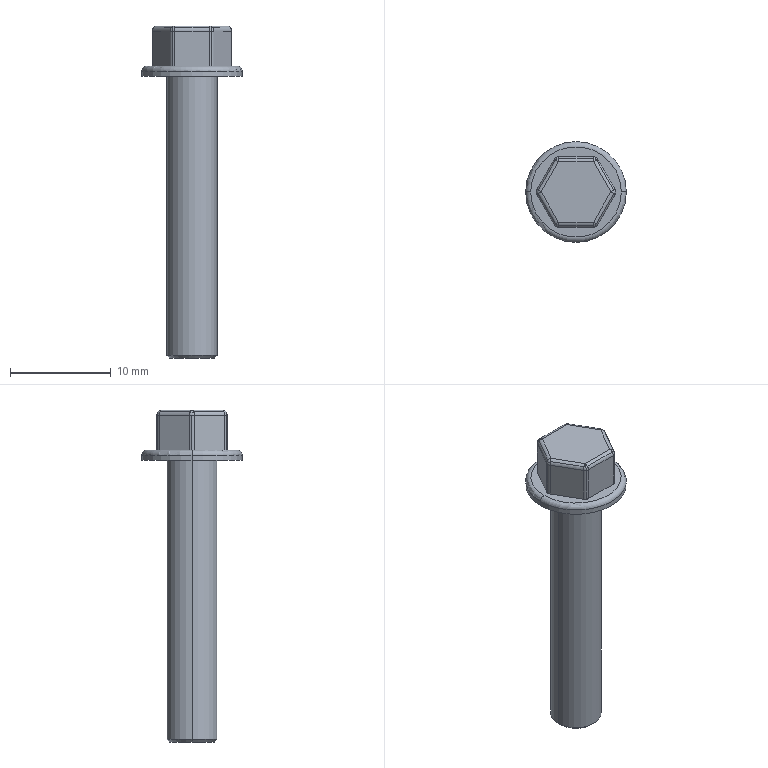Part | SolidWorks | features BaseBody 1 | 1 solid | 54 faces | box 10 x 10 x 33 mm | volume 794.369 mm3 | cylinder 28 | sphere 12 | plane 10 | cone 2 | torus 2 | commonest cylinder face diameters 1 x24 5 x2 10 x2
STEP:
#1=CARTESIAN_POINT('',(2.25,0.,-28.));
#2=VERTEX_POINT('',#1);
#3=CARTESIAN_POINT('',(-2.25,0.,-28.));
#4=VERTEX_POINT('',#3);
#5=CARTESIAN_POINT('',(0.,0.,-28.));
#6=DIRECTION('',(0.,0.,1.));
#7=DIRECTION('',(1.,0.,0.));
#8=AXIS2_PLACEMENT_3D('',#5,#6,#7);
#9=CIRCLE('',#8,2.25);
#10=EDGE_CURVE('',#2,#4,#9,.T.);
#11=ORIENTED_EDGE('',*,*,#10,.T.);
#12=CARTESIAN_POINT('',(-2.5,0.,-27.75));
#13=VERTEX_POINT('',#12);
#14=CARTESIAN_POINT('',(-2.375,0.,-27.875));
#15=DIRECTION('',(-0.7071,0.,0.7071));
#16=VECTOR('',#15,1000.);
#17=LINE('',#14,#16);
#18=EDGE_CURVE('',#4,#13,#17,.T.);
#19=ORIENTED_EDGE('',*,*,#18,.T.);
#20=CARTESIAN_POINT('',(2.5,0.,-27.75));
#21=VERTEX_POINT('',#20);
#22=CARTESIAN_POINT('',(0.,0.,-27.75));
#23=DIRECTION('',(0.,0.,-1.));
#24=DIRECTION('',(1.,0.,0.));
#25=AXIS2_PLACEMENT_3D('',#22,#23,#24);
#26=CIRCLE('',#25,2.5);
#27=EDGE_CURVE('',#13,#21,#26,.T.);
#28=ORIENTED_EDGE('',*,*,#27,.T.);
#29=CARTESIAN_POINT('',(2.375,0.,-27.875));
#30=DIRECTION('',(0.7071,0.,0.7071));
#31=VECTOR('',#30,1000.);
#32=LINE('',#29,#31);
#33=EDGE_CURVE('',#2,#21,#32,.T.);
#34=ORIENTED_EDGE('',*,*,#33,.F.);
#35=EDGE_LOOP('',(#11,#19,#28,#34));
#36=FACE_OUTER_BOUND('',#35,.T.);
#37=CARTESIAN_POINT('',(0.,0.,-27.875));
#38=DIRECTION('',(0.,0.,1.));
#39=DIRECTION('',(1.,0.,0.));
#40=AXIS2_PLACEMENT_3D('',#37,#38,#39);
#41=CONICAL_SURFACE('',#40,2.375,0.7854);
#42=ADVANCED_FACE('',(#36),#41,.T.);
#43=ORIENTED_EDGE('',*,*,#27,.F.);
#44=CARTESIAN_POINT('',(-2.5,0.,0.));
#45=VERTEX_POINT('',#44);
#46=CARTESIAN_POINT('',(-2.5,0.,0.));
#47=DIRECTION('',(0.,0.,1.));
#48=VECTOR('',#47,1000.);
#49=LINE('',#46,#48);
#50=EDGE_CURVE('',#13,#45,#49,.T.);
#51=ORIENTED_EDGE('',*,*,#50,.T.);
#52=CARTESIAN_POINT('',(2.5,0.,0.));
#53=VERTEX_POINT('',#52);
#54=CARTESIAN_POINT('',(0.,0.,0.));
#55=DIRECTION('',(0.,0.,1.));
#56=DIRECTION('',(1.,0.,0.));
#57=AXIS2_PLACEMENT_3D('',#54,#55,#56);
#58=CIRCLE('',#57,2.5);
#59=EDGE_CURVE('',#53,#45,#58,.T.);
#60=ORIENTED_EDGE('',*,*,#59,.F.);
#61=CARTESIAN_POINT('',(2.5,0.,0.));
#62=DIRECTION('',(0.,0.,1.));
#63=VECTOR('',#62,1000.);
#64=LINE('',#61,#63);
#65=EDGE_CURVE('',#21,#53,#64,.T.);
#66=ORIENTED_EDGE('',*,*,#65,.F.);
#67=EDGE_LOOP('',(#43,#51,#60,#66));
#68=FACE_OUTER_BOUND('',#67,.T.);
#69=CARTESIAN_POINT('',(0.,0.,0.));
#70=DIRECTION('',(0.,0.,1.));
#71=DIRECTION('',(1.,0.,0.));
#72=AXIS2_PLACEMENT_3D('',#69,#70,#71);
#73=CYLINDRICAL_SURFACE('',#72,2.5);
#74=ADVANCED_FACE('',(#68),#73,.T.);
#75=CARTESIAN_POINT('',(-1.918,-3.464,4.5));
#76=VERTEX_POINT('',#75);
#77=CARTESIAN_POINT('',(-1.982,-3.433,4.5));
#78=VERTEX_POINT('',#77);
#79=CARTESIAN_POINT('',(-1.732,-3.,4.5));
#80=DIRECTION('',(0.,0.,-1.));
#81=DIRECTION('',(0.,-1.,0.));
#82=AXIS2_PLACEMENT_3D('',#79,#80,#81);
#83=CIRCLE('',#82,0.5);
#84=EDGE_CURVE('',#76,#78,#83,.T.);
#85=ORIENTED_EDGE('',*,*,#84,.F.);
#86=CARTESIAN_POINT('',(-1.893,-3.093,4.964));
#87=VERTEX_POINT('',#86);
#88=CARTESIAN_POINT('',(-1.732,-3.,4.5));
#89=DIRECTION('',(-0.9014,0.3603,-0.2402));
#90=DIRECTION('',(-0.3712,-0.9286,0.));
#91=AXIS2_PLACEMENT_3D('',#88,#89,#90);
#92=CIRCLE('',#91,0.5);
#93=EDGE_CURVE('',#76,#87,#92,.T.);
#94=ORIENTED_EDGE('',*,*,#93,.T.);
#95=CARTESIAN_POINT('',(-2.038,-3.177,4.854));
#96=VERTEX_POINT('',#95);
#97=CARTESIAN_POINT('',(-1.732,-3.,4.5));
#98=DIRECTION('',(-0.5,0.866,0.));
#99=DIRECTION('',(-0.866,-0.5,0.));
#100=AXIS2_PLACEMENT_3D('',#97,#98,#99);
#101=CIRCLE('',#100,0.5);
#102=EDGE_CURVE('',#96,#87,#101,.T.);
#103=ORIENTED_EDGE('',*,*,#102,.F.);
#104=CARTESIAN_POINT('',(-2.165,-3.25,4.5));
#105=VERTEX_POINT('',#104);
#106=CARTESIAN_POINT('',(-1.732,-3.,4.5));
#107=DIRECTION('',(-0.5,0.866,0.));
#108=DIRECTION('',(-0.866,-0.5,0.));
#109=AXIS2_PLACEMENT_3D('',#106,#107,#108);
#110=CIRCLE('',#109,0.5);
#111=EDGE_CURVE('',#105,#96,#110,.T.);
#112=ORIENTED_EDGE('',*,*,#111,.F.);
#113=CARTESIAN_POINT('',(-1.732,-3.,4.5));
#114=DIRECTION('',(0.,0.,-1.));
#115=DIRECTION('',(0.,-1.,0.));
#116=AXIS2_PLACEMENT_3D('',#113,#114,#115);
#117=CIRCLE('',#116,0.5);
#118=EDGE_CURVE('',#78,#105,#117,.T.);
#119=ORIENTED_EDGE('',*,*,#118,.F.);
#120=EDGE_LOOP('',(#85,#94,#103,#112,#119));
#121=FACE_OUTER_BOUND('',#120,.T.);
#122=CARTESIAN_POINT('',(-1.732,-3.,4.5));
#123=DIRECTION('',(0.9014,-0.3603,0.2402));
#124=DIRECTION('',(-0.433,-0.75,0.5));
#125=AXIS2_PLACEMENT_3D('',#122,#123,#124);
#126=SPHERICAL_SURFACE('',#125,0.5);
#127=ADVANCED_FACE('',(#121),#126,.T.);
#128=CARTESIAN_POINT('',(-1.732,-3.5,4.5));
#129=VERTEX_POINT('',#128);
#130=CARTESIAN_POINT('',(-1.732,-3.,4.5));
#131=DIRECTION('',(0.,0.,-1.));
#132=DIRECTION('',(0.,-1.,0.));
#133=AXIS2_PLACEMENT_3D('',#130,#131,#132);
#134=CIRCLE('',#133,0.5);
#135=EDGE_CURVE('',#129,#76,#134,.T.);
#136=ORIENTED_EDGE('',*,*,#135,.T.);
#137=ORIENTED_EDGE('',*,*,#84,.T.);
#138=CARTESIAN_POINT('',(-1.982,-3.433,1.));
#139=VERTEX_POINT('',#138);
#140=CARTESIAN_POINT('',(-1.982,-3.433,1.));
#141=DIRECTION('',(0.,0.,-1.));
#142=VECTOR('',#141,1000.);
#143=LINE('',#140,#142);
#144=EDGE_CURVE('',#78,#139,#143,.T.);
#145=ORIENTED_EDGE('',*,*,#144,.T.);
#146=CARTESIAN_POINT('',(-1.732,-3.5,1.));
#147=VERTEX_POINT('',#146);
#148=CARTESIAN_POINT('',(-1.732,-3.,1.));
#149=DIRECTION('',(0.,0.,1.));
#150=DIRECTION('',(-0.5,-0.866,0.));
#151=AXIS2_PLACEMENT_3D('',#148,#149,#150);
#152=CIRCLE('',#151,0.5);
#153=EDGE_CURVE('',#139,#147,#152,.T.);
#154=ORIENTED_EDGE('',*,*,#153,.T.);
#155=CARTESIAN_POINT('',(-1.732,-3.5,1.));
#156=DIRECTION('',(0.,0.,1.));
#157=VECTOR('',#156,1000.);
#158=LINE('',#155,#157);
#159=EDGE_CURVE('',#147,#129,#158,.T.);
#160=ORIENTED_EDGE('',*,*,#159,.T.);
#161=EDGE_LOOP('',(#136,#137,#145,#154,#160));
#162=FACE_OUTER_BOUND('',#161,.T.);
#163=CARTESIAN_POINT('',(-1.732,-3.,1.));
#164=DIRECTION('',(0.,0.,-1.));
#165=DIRECTION('',(-0.5,-0.866,0.));
#166=AXIS2_PLACEMENT_3D('',#163,#164,#165);
#167=CYLINDRICAL_SURFACE('',#166,0.5);
#168=ADVANCED_FACE('',(#162),#167,.T.);
#169=CARTESIAN_POINT('',(1.918,-3.464,4.5));
#170=VERTEX_POINT('',#169);
#171=CARTESIAN_POINT('',(1.732,-3.5,4.5));
#172=VERTEX_POINT('',#171);
#173=CARTESIAN_POINT('',(1.732,-3.,4.5));
#174=DIRECTION('',(0.,0.,-1.));
#175=DIRECTION('',(0.866,-0.5,0.));
#176=AXIS2_PLACEMENT_3D('',#173,#174,#175);
#177=CIRCLE('',#176,0.5);
#178=EDGE_CURVE('',#170,#172,#177,.T.);
#179=ORIENTED_EDGE('',*,*,#178,.F.);
#180=CARTESIAN_POINT('',(1.893,-3.093,4.964));
#181=VERTEX_POINT('',#180);
#182=CARTESIAN_POINT('',(1.732,-3.,4.5));
#183=DIRECTION('',(-0.9014,-0.3603,0.2402));
#184=DIRECTION('',(0.3712,-0.9286,0.));
#185=AXIS2_PLACEMENT_3D('',#182,#183,#184);
#186=CIRCLE('',#185,0.5);
#187=EDGE_CURVE('',#170,#181,#186,.T.);
#188=ORIENTED_EDGE('',*,*,#187,.T.);
#189=CARTESIAN_POINT('',(1.732,-3.,5.));
#190=VERTEX_POINT('',#189);
#191=CARTESIAN_POINT('',(1.732,-3.,4.5));
#192=DIRECTION('',(0.5,0.866,0.));
#193=DIRECTION('',(0.,0.,1.));
#194=AXIS2_PLACEMENT_3D('',#191,#192,#193);
#195=CIRCLE('',#194,0.5);
#196=EDGE_CURVE('',#190,#181,#195,.T.);
#197=ORIENTED_EDGE('',*,*,#196,.F.);
#198=CARTESIAN_POINT('',(1.732,-3.354,4.854));
#199=VERTEX_POINT('',#198);
#200=CARTESIAN_POINT('',(1.732,-3.,4.5));
#201=DIRECTION('',(-1.,0.,0.));
#202=DIRECTION('',(0.,-1.,0.));
#203=AXIS2_PLACEMENT_3D('',#200,#201,#202);
#204=CIRCLE('',#203,0.5);
#205=EDGE_CURVE('',#199,#190,#204,.T.);
#206=ORIENTED_EDGE('',*,*,#205,.F.);
#207=CARTESIAN_POINT('',(1.732,-3.,4.5));
#208=DIRECTION('',(-1.,0.,0.));
#209=DIRECTION('',(0.,-1.,0.));
#210=AXIS2_PLACEMENT_3D('',#207,#208,#209);
#211=CIRCLE('',#210,0.5);
#212=EDGE_CURVE('',#172,#199,#211,.T.);
#213=ORIENTED_EDGE('',*,*,#212,.F.);
#214=EDGE_LOOP('',(#179,#188,#197,#206,#213));
#215=FACE_OUTER_BOUND('',#214,.T.);
#216=CARTESIAN_POINT('',(1.732,-3.,4.5));
#217=DIRECTION('',(0.9014,0.3603,-0.2402));
#218=DIRECTION('',(0.433,-0.75,0.5));
#219=AXIS2_PLACEMENT_3D('',#216,#217,#218);
#220=SPHERICAL_SURFACE('',#219,0.5);
#221=ADVANCED_FACE('',(#215),#220,.T.);
#222=CARTESIAN_POINT('',(2.165,-3.25,4.5));
#223=VERTEX_POINT('',#222);
#224=CARTESIAN_POINT('',(1.982,-3.433,4.5));
#225=VERTEX_POINT('',#224);
#226=CARTESIAN_POINT('',(1.732,-3.,4.5));
#227=DIRECTION('',(0.,0.,-1.));
#228=DIRECTION('',(0.866,-0.5,0.));
#229=AXIS2_PLACEMENT_3D('',#226,#227,#228);
#230=CIRCLE('',#229,0.5);
#231=EDGE_CURVE('',#223,#225,#230,.T.);
#232=ORIENTED_EDGE('',*,*,#231,.T.);
#233=CARTESIAN_POINT('',(1.982,-3.433,1.));
#234=VERTEX_POINT('',#233);
#235=CARTESIAN_POINT('',(1.982,-3.433,1.));
#236=DIRECTION('',(0.,0.,-1.));
#237=VECTOR('',#236,1000.);
#238=LINE('',#235,#237);
#239=EDGE_CURVE('',#225,#234,#238,.T.);
#240=ORIENTED_EDGE('',*,*,#239,.T.);
#241=CARTESIAN_POINT('',(2.165,-3.25,1.));
#242=VERTEX_POINT('',#241);
#243=CARTESIAN_POINT('',(1.732,-3.,1.));
#244=DIRECTION('',(0.,0.,1.));
#245=DIRECTION('',(0.5,-0.866,0.));
#246=AXIS2_PLACEMENT_3D('',#243,#244,#245);
#247=CIRCLE('',#246,0.5);
#248=EDGE_CURVE('',#234,#242,#247,.T.);
#249=ORIENTED_EDGE('',*,*,#248,.T.);
#250=CARTESIAN_POINT('',(2.165,-3.25,1.));
#251=DIRECTION('',(0.,0.,1.));
#252=VECTOR('',#251,1000.);
#253=LINE('',#250,#252);
#254=EDGE_CURVE('',#242,#223,#253,.T.);
#255=ORIENTED_EDGE('',*,*,#254,.T.);
#256=EDGE_LOOP('',(#232,#240,#249,#255));
#257=FACE_OUTER_BOUND('',#256,.T.);
#258=CARTESIAN_POINT('',(1.732,-3.,1.));
#259=DIRECTION('',(0.,0.,-1.));
#260=DIRECTION('',(0.5,-0.866,0.));
#261=AXIS2_PLACEMENT_3D('',#258,#259,#260);
#262=CYLINDRICAL_SURFACE('',#261,0.5);
#263=ADVANCED_FACE('',(#257),#262,.T.);
#264=CARTESIAN_POINT('',(-3.851,-0.2236,4.724));
#265=VERTEX_POINT('',#264);
#266=CARTESIAN_POINT('',(-3.897,-0.25,4.5));
#267=VERTEX_POINT('',#266);
#268=CARTESIAN_POINT('',(-3.464,0.,4.5));
#269=DIRECTION('',(0.5,-0.866,0.));
#270=DIRECTION('',(0.,0.,1.));
#271=AXIS2_PLACEMENT_3D('',#268,#269,#270);
#272=CIRCLE('',#271,0.5);
#273=EDGE_CURVE('',#265,#267,#272,.T.);
#274=ORIENTED_EDGE('',*,*,#273,.F.);
#275=CARTESIAN_POINT('',(-3.851,0.2236,4.724));
#276=VERTEX_POINT('',#275);
#277=CARTESIAN_POINT('',(-3.464,0.,4.5));
#278=DIRECTION('',(-0.5,0.,-0.866));
#279=DIRECTION('',(-0.866,0.,0.5));
#280=AXIS2_PLACEMENT_3D('',#277,#278,#279);
#281=CIRCLE('',#280,0.5);
#282=EDGE_CURVE('',#265,#276,#281,.T.);
#283=ORIENTED_EDGE('',*,*,#282,.T.);
#284=CARTESIAN_POINT('',(-3.897,0.25,4.5));
#285=VERTEX_POINT('',#284);
#286=CARTESIAN_POINT('',(-3.464,0.,4.5));
#287=DIRECTION('',(0.5,0.866,0.));
#288=DIRECTION('',(-0.866,0.5,0.));
#289=AXIS2_PLACEMENT_3D('',#286,#287,#288);
#290=CIRCLE('',#289,0.5);
#291=EDGE_CURVE('',#285,#276,#290,.T.);
#292=ORIENTED_EDGE('',*,*,#291,.F.);
#293=CARTESIAN_POINT('',(-3.964,0.,4.5));
#294=VERTEX_POINT('',#293);
#295=CARTESIAN_POINT('',(-3.464,0.,4.5));
#296=DIRECTION('',(0.,0.,-1.));
#297=DIRECTION('',(-0.866,-0.5,0.));
#298=AXIS2_PLACEMENT_3D('',#295,#296,#297);
#299=CIRCLE('',#298,0.5);
#300=EDGE_CURVE('',#294,#285,#299,.T.);
#301=ORIENTED_EDGE('',*,*,#300,.F.);
#302=CARTESIAN_POINT('',(-3.464,0.,4.5));
#303=DIRECTION('',(0.,0.,-1.));
#304=DIRECTION('',(-0.866,-0.5,0.));
#305=AXIS2_PLACEMENT_3D('',#302,#303,#304);
#306=CIRCLE('',#305,0.5);
#307=EDGE_CURVE('',#267,#294,#306,.T.);
#308=ORIENTED_EDGE('',*,*,#307,.F.);
#309=EDGE_LOOP('',(#274,#283,#292,#301,#308));
#310=FACE_OUTER_BOUND('',#309,.T.);
#311=CARTESIAN_POINT('',(-3.464,0.,4.5));
#312=DIRECTION('',(0.5,0.,0.866));
#313=DIRECTION('',(-0.866,0.,0.5));
#314=AXIS2_PLACEMENT_3D('',#311,#312,#313);
#315=SPHERICAL_SURFACE('',#314,0.5);
#316=ADVANCED_FACE('',(#310),#315,.T.);
#317=ORIENTED_EDGE('',*,*,#307,.T.);
#318=CARTESIAN_POINT('',(-3.964,0.,1.));
#319=VERTEX_POINT('',#318);
#320=CARTESIAN_POINT('',(-3.964,0.,1.));
#321=DIRECTION('',(0.,0.,-1.));
#322=VECTOR('',#321,1000.);
#323=LINE('',#320,#322);
#324=EDGE_CURVE('',#294,#319,#323,.T.);
#325=ORIENTED_EDGE('',*,*,#324,.T.);
#326=CARTESIAN_POINT('',(-3.897,-0.25,1.));
#327=VERTEX_POINT('',#326);
#328=CARTESIAN_POINT('',(-3.464,0.,1.));
#329=DIRECTION('',(0.,0.,1.));
#330=DIRECTION('',(-1.,0.,0.));
#331=AXIS2_PLACEMENT_3D('',#328,#329,#330);
#332=CIRCLE('',#331,0.5);
#333=EDGE_CURVE('',#319,#327,#332,.T.);
#334=ORIENTED_EDGE('',*,*,#333,.T.);
#335=CARTESIAN_POINT('',(-3.897,-0.25,1.));
#336=DIRECTION('',(0.,0.,1.));
#337=VECTOR('',#336,1000.);
#338=LINE('',#335,#337);
#339=EDGE_CURVE('',#327,#267,#338,.T.);
#340=ORIENTED_EDGE('',*,*,#339,.T.);
#341=EDGE_LOOP('',(#317,#325,#334,#340));
#342=FACE_OUTER_BOUND('',#341,.T.);
#343=CARTESIAN_POINT('',(-3.464,0.,1.));
#344=DIRECTION('',(0.,0.,-1.));
#345=DIRECTION('',(-1.,0.,0.));
#346=AXIS2_PLACEMENT_3D('',#343,#344,#345);
#347=CYLINDRICAL_SURFACE('',#346,0.5);
#348=ADVANCED_FACE('',(#342),#347,.T.);
#349=ORIENTED_EDGE('',*,*,#111,.T.);
#350=CARTESIAN_POINT('',(-3.77,-0.1768,4.854));
#351=VERTEX_POINT('',#350);
#352=CARTESIAN_POINT('',(-3.409,-0.8018,4.854));
#353=DIRECTION('',(-0.5,0.866,0.));
#354=VECTOR('',#353,1000.);
#355=LINE('',#352,#354);
#356=EDGE_CURVE('',#96,#351,#355,.T.);
#357=ORIENTED_EDGE('',*,*,#356,.T.);
#358=CARTESIAN_POINT('',(-3.464,0.,4.5));
#359=DIRECTION('',(0.5,-0.866,0.));
#360=DIRECTION('',(0.,0.,1.));
#361=AXIS2_PLACEMENT_3D('',#358,#359,#360);
#362=CIRCLE('',#361,0.5);
#363=EDGE_CURVE('',#351,#265,#362,.T.);
#364=ORIENTED_EDGE('',*,*,#363,.T.);
#365=ORIENTED_EDGE('',*,*,#273,.T.);
#366=CARTESIAN_POINT('',(-3.536,-0.875,4.5));
#367=DIRECTION('',(0.5,-0.866,0.));
#368=VECTOR('',#367,1000.);
#369=LINE('',#366,#368);
#370=EDGE_CURVE('',#267,#105,#369,.T.);
#371=ORIENTED_EDGE('',*,*,#370,.T.);
#372=EDGE_LOOP('',(#349,#357,#364,#365,#371));
#373=FACE_OUTER_BOUND('',#372,.T.);
#374=CARTESIAN_POINT('',(-3.103,-0.625,4.5));
#375=DIRECTION('',(-0.5,0.866,0.));
#376=DIRECTION('',(-0.6124,-0.3536,0.7071));
#377=AXIS2_PLACEMENT_3D('',#374,#375,#376);
#378=CYLINDRICAL_SURFACE('',#377,0.5);
#379=ADVANCED_FACE('',(#373),#378,.T.);
#380=CARTESIAN_POINT('',(3.851,0.2236,4.724));
#381=VERTEX_POINT('',#380);
#382=CARTESIAN_POINT('',(3.897,0.25,4.5));
#383=VERTEX_POINT('',#382);
#384=CARTESIAN_POINT('',(3.464,0.,4.5));
#385=DIRECTION('',(-0.5,0.866,0.));
#386=DIRECTION('',(0.,0.,1.));
#387=AXIS2_PLACEMENT_3D('',#384,#385,#386);
#388=CIRCLE('',#387,0.5);
#389=EDGE_CURVE('',#381,#383,#388,.T.);
#390=ORIENTED_EDGE('',*,*,#389,.F.);
#391=CARTESIAN_POINT('',(3.851,-0.2236,4.724));
#392=VERTEX_POINT('',#391);
#393=CARTESIAN_POINT('',(3.464,0.,4.5));
#394=DIRECTION('',(0.5,0.,-0.866));
#395=DIRECTION('',(-0.866,0.,-0.5));
#396=AXIS2_PLACEMENT_3D('',#393,#394,#395);
#397=CIRCLE('',#396,0.5);
#398=EDGE_CURVE('',#381,#392,#397,.T.);
#399=ORIENTED_EDGE('',*,*,#398,.T.);
#400=CARTESIAN_POINT('',(3.897,-0.25,4.5));
#401=VERTEX_POINT('',#400);
#402=CARTESIAN_POINT('',(3.464,0.,4.5));
#403=DIRECTION('',(-0.5,-0.866,0.));
#404=DIRECTION('',(0.866,-0.5,0.));
#405=AXIS2_PLACEMENT_3D('',#402,#403,#404);
#406=CIRCLE('',#405,0.5);
#407=EDGE_CURVE('',#401,#392,#406,.T.);
#408=ORIENTED_EDGE('',*,*,#407,.F.);
#409=CARTESIAN_POINT('',(3.964,0.,4.5));
#410=VERTEX_POINT('',#409);
#411=CARTESIAN_POINT('',(3.464,0.,4.5));
#412=DIRECTION('',(0.,0.,-1.));
#413=DIRECTION('',(0.866,0.5,0.));
#414=AXIS2_PLACEMENT_3D('',#411,#412,#413);
#415=CIRCLE('',#414,0.5);
#416=EDGE_CURVE('',#410,#401,#415,.T.);
#417=ORIENTED_EDGE('',*,*,#416,.F.);
#418=CARTESIAN_POINT('',(3.464,0.,4.5));
#419=DIRECTION('',(0.,0.,-1.));
#420=DIRECTION('',(0.866,0.5,0.));
#421=AXIS2_PLACEMENT_3D('',#418,#419,#420);
#422=CIRCLE('',#421,0.5);
#423=EDGE_CURVE('',#383,#410,#422,.T.);
#424=ORIENTED_EDGE('',*,*,#423,.F.);
#425=EDGE_LOOP('',(#390,#399,#408,#417,#424));
#426=FACE_OUTER_BOUND('',#425,.T.);
#427=CARTESIAN_POINT('',(3.464,0.,4.5));
#428=DIRECTION('',(-0.5,0.,0.866));
#429=DIRECTION('',(0.866,0.,0.5));
#430=AXIS2_PLACEMENT_3D('',#427,#428,#429);
#431=SPHERICAL_SURFACE('',#430,0.5);
#432=ADVANCED_FACE('',(#426),#431,.T.);
#433=ORIENTED_EDGE('',*,*,#423,.T.);
#434=CARTESIAN_POINT('',(3.964,0.,1.));
#435=VERTEX_POINT('',#434);
#436=CARTESIAN_POINT('',(3.964,0.,1.));
#437=DIRECTION('',(0.,0.,-1.));
#438=VECTOR('',#437,1000.);
#439=LINE('',#436,#438);
#440=EDGE_CURVE('',#410,#435,#439,.T.);
#441=ORIENTED_EDGE('',*,*,#440,.T.);
#442=CARTESIAN_POINT('',(3.897,0.25,1.));
#443=VERTEX_POINT('',#442);
#444=CARTESIAN_POINT('',(3.464,0.,1.));
#445=DIRECTION('',(0.,0.,1.));
#446=DIRECTION('',(1.,0.,0.));
#447=AXIS2_PLACEMENT_3D('',#444,#445,#446);
#448=CIRCLE('',#447,0.5);
#449=EDGE_CURVE('',#435,#443,#448,.T.);
#450=ORIENTED_EDGE('',*,*,#449,.T.);
#451=CARTESIAN_POINT('',(3.897,0.25,1.));
#452=DIRECTION('',(0.,0.,1.));
#453=VECTOR('',#452,1000.);
#454=LINE('',#451,#453);
#455=EDGE_CURVE('',#443,#383,#454,.T.);
#456=ORIENTED_EDGE('',*,*,#455,.T.);
#457=EDGE_LOOP('',(#433,#441,#450,#456));
#458=FACE_OUTER_BOUND('',#457,.T.);
#459=CARTESIAN_POINT('',(3.464,0.,1.));
#460=DIRECTION('',(0.,0.,-1.));
#461=DIRECTION('',(1.,0.,0.));
#462=AXIS2_PLACEMENT_3D('',#459,#460,#461);
#463=CYLINDRICAL_SURFACE('',#462,0.5);
#464=ADVANCED_FACE('',(#458),#463,.T.);
#465=CARTESIAN_POINT('',(-1.893,3.093,4.964));
#466=VERTEX_POINT('',#465);
#467=CARTESIAN_POINT('',(-2.038,3.177,4.854));
#468=VERTEX_POINT('',#467);
#469=CARTESIAN_POINT('',(-1.732,3.,4.5));
#470=DIRECTION('',(-0.5,-0.866,0.));
#471=DIRECTION('',(0.,0.,1.));
#472=AXIS2_PLACEMENT_3D('',#469,#470,#471);
#473=CIRCLE('',#472,0.5);
#474=EDGE_CURVE('',#466,#468,#473,.T.);
#475=ORIENTED_EDGE('',*,*,#474,.F.);
#476=CARTESIAN_POINT('',(-1.918,3.464,4.5));
#477=VERTEX_POINT('',#476);
#478=CARTESIAN_POINT('',(-1.732,3.,4.5));
#479=DIRECTION('',(-0.9014,-0.3603,-0.2402));
#480=DIRECTION('',(0.3712,-0.9286,0.));
#481=AXIS2_PLACEMENT_3D('',#478,#479,#480);
#482=CIRCLE('',#481,0.5);
#483=EDGE_CURVE('',#466,#477,#482,.T.);
#484=ORIENTED_EDGE('',*,*,#483,.T.);
#485=CARTESIAN_POINT('',(-1.982,3.433,4.5));
#486=VERTEX_POINT('',#485);
#487=CARTESIAN_POINT('',(-1.732,3.,4.5));
#488=DIRECTION('',(0.,0.,-1.));
#489=DIRECTION('',(-0.866,0.5,0.));
#490=AXIS2_PLACEMENT_3D('',#487,#488,#489);
#491=CIRCLE('',#490,0.5);
#492=EDGE_CURVE('',#486,#477,#491,.T.);
#493=ORIENTED_EDGE('',*,*,#492,.F.);
#494=CARTESIAN_POINT('',(-2.165,3.25,4.5));
#495=VERTEX_POINT('',#494);
#496=CARTESIAN_POINT('',(-1.732,3.,4.5));
#497=DIRECTION('',(0.,0.,-1.));
#498=DIRECTION('',(-0.866,0.5,0.));
#499=AXIS2_PLACEMENT_3D('',#496,#497,#498);
#500=CIRCLE('',#499,0.5);
#501=EDGE_CURVE('',#495,#486,#500,.T.);
#502=ORIENTED_EDGE('',*,*,#501,.F.);
#503=CARTESIAN_POINT('',(-1.732,3.,4.5));
#504=DIRECTION('',(-0.5,-0.866,0.));
#505=DIRECTION('',(0.,0.,1.));
#506=AXIS2_PLACEMENT_3D('',#503,#504,#505);
#507=CIRCLE('',#506,0.5);
#508=EDGE_CURVE('',#468,#495,#507,.T.);
#509=ORIENTED_EDGE('',*,*,#508,.F.);
#510=EDGE_LOOP('',(#475,#484,#493,#502,#509));
#511=FACE_OUTER_BOUND('',#510,.T.);
#512=CARTESIAN_POINT('',(-1.732,3.,4.5));
#513=DIRECTION('',(0.9014,0.3603,0.2402));
#514=DIRECTION('',(-0.433,0.75,0.5));
#515=AXIS2_PLACEMENT_3D('',#512,#513,#514);
#516=SPHERICAL_SURFACE('',#515,0.5);
#517=ADVANCED_FACE('',(#511),#516,.T.);
#518=ORIENTED_EDGE('',*,*,#501,.T.);
#519=CARTESIAN_POINT('',(-1.982,3.433,1.));
#520=VERTEX_POINT('',#519);
#521=CARTESIAN_POINT('',(-1.982,3.433,1.));
#522=DIRECTION('',(0.,0.,-1.));
#523=VECTOR('',#522,1000.);
#524=LINE('',#521,#523);
#525=EDGE_CURVE('',#486,#520,#524,.T.);
#526=ORIENTED_EDGE('',*,*,#525,.T.);
#527=CARTESIAN_POINT('',(-2.165,3.25,1.));
#528=VERTEX_POINT('',#527);
#529=CARTESIAN_POINT('',(-1.732,3.,1.));
#530=DIRECTION('',(0.,0.,1.));
#531=DIRECTION('',(-0.5,0.866,0.));
#532=AXIS2_PLACEMENT_3D('',#529,#530,#531);
#533=CIRCLE('',#532,0.5);
#534=EDGE_CURVE('',#520,#528,#533,.T.);
#535=ORIENTED_EDGE('',*,*,#534,.T.);
#536=CARTESIAN_POINT('',(-2.165,3.25,1.));
#537=DIRECTION('',(0.,0.,1.));
#538=VECTOR('',#537,1000.);
#539=LINE('',#536,#538);
#540=EDGE_CURVE('',#528,#495,#539,.T.);
#541=ORIENTED_EDGE('',*,*,#540,.T.);
#542=EDGE_LOOP('',(#518,#526,#535,#541));
#543=FACE_OUTER_BOUND('',#542,.T.);
#544=CARTESIAN_POINT('',(-1.732,3.,1.));
#545=DIRECTION('',(0.,0.,-1.));
#546=DIRECTION('',(-0.5,0.866,0.));
#547=AXIS2_PLACEMENT_3D('',#544,#545,#546);
#548=CYLINDRICAL_SURFACE('',#547,0.5);
#549=ADVANCED_FACE('',(#543),#548,.T.);
#550=ORIENTED_EDGE('',*,*,#291,.T.);
#551=CARTESIAN_POINT('',(-3.77,0.1768,4.854));
#552=VERTEX_POINT('',#551);
#553=CARTESIAN_POINT('',(-3.464,0.,4.5));
#554=DIRECTION('',(0.5,0.866,0.));
#555=DIRECTION('',(-0.866,0.5,0.));
#556=AXIS2_PLACEMENT_3D('',#553,#554,#555);
#557=CIRCLE('',#556,0.5);
#558=EDGE_CURVE('',#276,#552,#557,.T.);
#559=ORIENTED_EDGE('',*,*,#558,.T.);
#560=CARTESIAN_POINT('',(-2.399,2.552,4.854));
#561=DIRECTION('',(0.5,0.866,0.));
#562=VECTOR('',#561,1000.);
#563=LINE('',#560,#562);
#564=EDGE_CURVE('',#552,#468,#563,.T.);
#565=ORIENTED_EDGE('',*,*,#564,.T.);
#566=ORIENTED_EDGE('',*,*,#508,.T.);
#567=CARTESIAN_POINT('',(-2.526,2.625,4.5));
#568=DIRECTION('',(-0.5,-0.866,0.));
#569=VECTOR('',#568,1000.);
#570=LINE('',#567,#569);
#571=EDGE_CURVE('',#495,#285,#570,.T.);
#572=ORIENTED_EDGE('',*,*,#571,.T.);
#573=EDGE_LOOP('',(#550,#559,#565,#566,#572));
#574=FACE_OUTER_BOUND('',#573,.T.);
#575=CARTESIAN_POINT('',(-2.093,2.375,4.5));
#576=DIRECTION('',(0.5,0.866,0.));
#577=DIRECTION('',(-0.6124,0.3536,0.7071));
#578=AXIS2_PLACEMENT_3D('',#575,#576,#577);
#579=CYLINDRICAL_SURFACE('',#578,0.5);
#580=ADVANCED_FACE('',(#574),#579,.T.);
#581=CARTESIAN_POINT('',(1.893,3.093,4.964));
#582=VERTEX_POINT('',#581);
#583=CARTESIAN_POINT('',(1.732,3.,5.));
#584=VERTEX_POINT('',#583);
#585=CARTESIAN_POINT('',(1.732,3.,4.5));
#586=DIRECTION('',(0.5,-0.866,0.));
#587=DIRECTION('',(0.866,0.5,0.));
#588=AXIS2_PLACEMENT_3D('',#585,#586,#587);
#589=CIRCLE('',#588,0.5);
#590=EDGE_CURVE('',#582,#584,#589,.T.);
#591=ORIENTED_EDGE('',*,*,#590,.F.);
#592=CARTESIAN_POINT('',(1.918,3.464,4.5));
#593=VERTEX_POINT('',#592);
#594=CARTESIAN_POINT('',(1.732,3.,4.5));
#595=DIRECTION('',(-0.9014,0.3603,0.2402));
#596=DIRECTION('',(-0.3712,-0.9286,0.));
#597=AXIS2_PLACEMENT_3D('',#594,#595,#596);
#598=CIRCLE('',#597,0.5);
#599=EDGE_CURVE('',#582,#593,#598,.T.);
#600=ORIENTED_EDGE('',*,*,#599,.T.);
#601=CARTESIAN_POINT('',(1.732,3.5,4.5));
#602=VERTEX_POINT('',#601);
#603=CARTESIAN_POINT('',(1.732,3.,4.5));
#604=DIRECTION('',(0.,0.,-1.));
#605=DIRECTION('',(0.,1.,0.));
#606=AXIS2_PLACEMENT_3D('',#603,#604,#605);
#607=CIRCLE('',#606,0.5);
#608=EDGE_CURVE('',#602,#593,#607,.T.);
#609=ORIENTED_EDGE('',*,*,#608,.F.);
#610=CARTESIAN_POINT('',(1.732,3.354,4.854));
#611=VERTEX_POINT('',#610);
#612=CARTESIAN_POINT('',(1.732,3.,4.5));
#613=DIRECTION('',(-1.,0.,0.));
#614=DIRECTION('',(0.,0.,1.));
#615=AXIS2_PLACEMENT_3D('',#612,#613,#614);
#616=CIRCLE('',#615,0.5);
#617=EDGE_CURVE('',#611,#602,#616,.T.);
#618=ORIENTED_EDGE('',*,*,#617,.F.);
#619=CARTESIAN_POINT('',(1.732,3.,4.5));
#620=DIRECTION('',(-1.,0.,0.));
#621=DIRECTION('',(0.,0.,1.));
#622=AXIS2_PLACEMENT_3D('',#619,#620,#621);
#623=CIRCLE('',#622,0.5);
#624=EDGE_CURVE('',#584,#611,#623,.T.);
#625=ORIENTED_EDGE('',*,*,#624,.F.);
#626=EDGE_LOOP('',(#591,#600,#609,#618,#625));
#627=FACE_OUTER_BOUND('',#626,.T.);
#628=CARTESIAN_POINT('',(1.732,3.,4.5));
#629=DIRECTION('',(0.9014,-0.3603,-0.2402));
#630=DIRECTION('',(0.433,0.75,0.5));
#631=AXIS2_PLACEMENT_3D('',#628,#629,#630);
#632=SPHERICAL_SURFACE('',#631,0.5);
#633=ADVANCED_FACE('',(#627),#632,.T.);
#634=ORIENTED_EDGE('',*,*,#608,.T.);
#635=CARTESIAN_POINT('',(1.982,3.433,4.5));
#636=VERTEX_POINT('',#635);
#637=CARTESIAN_POINT('',(1.732,3.,4.5));
#638=DIRECTION('',(0.,0.,-1.));
#639=DIRECTION('',(0.,1.,0.));
#640=AXIS2_PLACEMENT_3D('',#637,#638,#639);
#641=CIRCLE('',#640,0.5);
#642=EDGE_CURVE('',#593,#636,#641,.T.);
#643=ORIENTED_EDGE('',*,*,#642,.T.);
#644=CARTESIAN_POINT('',(1.982,3.433,1.));
#645=VERTEX_POINT('',#644);
#646=CARTESIAN_POINT('',(1.982,3.433,1.));
#647=DIRECTION('',(0.,0.,-1.));
#648=VECTOR('',#647,1000.);
#649=LINE('',#646,#648);
#650=EDGE_CURVE('',#636,#645,#649,.T.);
#651=ORIENTED_EDGE('',*,*,#650,.T.);
#652=CARTESIAN_POINT('',(1.732,3.5,1.));
#653=VERTEX_POINT('',#652);
#654=CARTESIAN_POINT('',(1.732,3.,1.));
#655=DIRECTION('',(0.,0.,1.));
#656=DIRECTION('',(0.5,0.866,0.));
#657=AXIS2_PLACEMENT_3D('',#654,#655,#656);
#658=CIRCLE('',#657,0.5);
#659=EDGE_CURVE('',#645,#653,#658,.T.);
#660=ORIENTED_EDGE('',*,*,#659,.T.);
#661=CARTESIAN_POINT('',(1.732,3.5,1.));
#662=DIRECTION('',(0.,0.,1.));
#663=VECTOR('',#662,1000.);
#664=LINE('',#661,#663);
#665=EDGE_CURVE('',#653,#602,#664,.T.);
#666=ORIENTED_EDGE('',*,*,#665,.T.);
#667=EDGE_LOOP('',(#634,#643,#651,#660,#666));
#668=FACE_OUTER_BOUND('',#667,.T.);
#669=CARTESIAN_POINT('',(1.732,3.,1.));
#670=DIRECTION('',(0.,0.,-1.));
#671=DIRECTION('',(0.5,0.866,0.));
#672=AXIS2_PLACEMENT_3D('',#669,#670,#671);
#673=CYLINDRICAL_SURFACE('',#672,0.5);
#674=ADVANCED_FACE('',(#668),#673,.T.);
#675=CARTESIAN_POINT('',(-1.732,3.5,4.5));
#676=VERTEX_POINT('',#675);
#677=CARTESIAN_POINT('',(-1.732,3.354,4.854));
#678=VERTEX_POINT('',#677);
#679=CARTESIAN_POINT('',(-1.732,3.,4.5));
#680=DIRECTION('',(1.,0.,0.));
#681=DIRECTION('',(0.,1.,0.));
#682=AXIS2_PLACEMENT_3D('',#679,#680,#681);
#683=CIRCLE('',#682,0.5);
#684=EDGE_CURVE('',#676,#678,#683,.T.);
#685=ORIENTED_EDGE('',*,*,#684,.T.);
#686=CARTESIAN_POINT('',(1.01,3.354,4.854));
#687=DIRECTION('',(1.,0.,0.));
#688=VECTOR('',#687,1000.);
#689=LINE('',#686,#688);
#690=EDGE_CURVE('',#678,#611,#689,.T.);
#691=ORIENTED_EDGE('',*,*,#690,.T.);
#692=ORIENTED_EDGE('',*,*,#617,.T.);
#693=CARTESIAN_POINT('',(1.01,3.5,4.5));
#694=DIRECTION('',(-1.,0.,0.));
#695=VECTOR('',#694,1000.);
#696=LINE('',#693,#695);
#697=EDGE_CURVE('',#602,#676,#696,.T.);
#698=ORIENTED_EDGE('',*,*,#697,.T.);
#699=EDGE_LOOP('',(#685,#691,#692,#698));
#700=FACE_OUTER_BOUND('',#699,.T.);
#701=CARTESIAN_POINT('',(1.01,3.,4.5));
#702=DIRECTION('',(1.,0.,0.));
#703=DIRECTION('',(0.,0.7071,0.7071));
#704=AXIS2_PLACEMENT_3D('',#701,#702,#703);
#705=CYLINDRICAL_SURFACE('',#704,0.5);
#706=ADVANCED_FACE('',(#700),#705,.T.);
#707=CARTESIAN_POINT('',(2.165,3.25,4.5));
#708=VERTEX_POINT('',#707);
#709=CARTESIAN_POINT('',(2.038,3.177,4.854));
#710=VERTEX_POINT('',#709);
#711=CARTESIAN_POINT('',(1.732,3.,4.5));
#712=DIRECTION('',(0.5,-0.866,0.));
#713=DIRECTION('',(0.866,0.5,0.));
#714=AXIS2_PLACEMENT_3D('',#711,#712,#713);
#715=CIRCLE('',#714,0.5);
#716=EDGE_CURVE('',#708,#710,#715,.T.);
#717=ORIENTED_EDGE('',*,*,#716,.T.);
#718=CARTESIAN_POINT('',(3.77,0.1768,4.854));
#719=VERTEX_POINT('',#718);
#720=CARTESIAN_POINT('',(3.409,0.8018,4.854));
#721=DIRECTION('',(0.5,-0.866,0.));
#722=VECTOR('',#721,1000.);
#723=LINE('',#720,#722);
#724=EDGE_CURVE('',#710,#719,#723,.T.);
#725=ORIENTED_EDGE('',*,*,#724,.T.);
#726=CARTESIAN_POINT('',(3.464,0.,4.5));
#727=DIRECTION('',(-0.5,0.866,0.));
#728=DIRECTION('',(0.,0.,1.));
#729=AXIS2_PLACEMENT_3D('',#726,#727,#728);
#730=CIRCLE('',#729,0.5);
#731=EDGE_CURVE('',#719,#381,#730,.T.);
#732=ORIENTED_EDGE('',*,*,#731,.T.);
#733=ORIENTED_EDGE('',*,*,#389,.T.);
#734=CARTESIAN_POINT('',(3.536,0.875,4.5));
#735=DIRECTION('',(-0.5,0.866,0.));
#736=VECTOR('',#735,1000.);
#737=LINE('',#734,#736);
#738=EDGE_CURVE('',#383,#708,#737,.T.);
#739=ORIENTED_EDGE('',*,*,#738,.T.);
#740=EDGE_LOOP('',(#717,#725,#732,#733,#739));
#741=FACE_OUTER_BOUND('',#740,.T.);
#742=CARTESIAN_POINT('',(3.103,0.625,4.5));
#743=DIRECTION('',(0.5,-0.866,0.));
#744=DIRECTION('',(0.6124,0.3536,0.7071));
#745=AXIS2_PLACEMENT_3D('',#742,#743,#744);
#746=CYLINDRICAL_SURFACE('',#745,0.5);
#747=ADVANCED_FACE('',(#741),#746,.T.);
#748=ORIENTED_EDGE('',*,*,#407,.T.);
#749=CARTESIAN_POINT('',(3.77,-0.1768,4.854));
#750=VERTEX_POINT('',#749);
#751=CARTESIAN_POINT('',(3.464,0.,4.5));
#752=DIRECTION('',(-0.5,-0.866,0.));
#753=DIRECTION('',(0.866,-0.5,0.));
#754=AXIS2_PLACEMENT_3D('',#751,#752,#753);
#755=CIRCLE('',#754,0.5);
#756=EDGE_CURVE('',#392,#750,#755,.T.);
#757=ORIENTED_EDGE('',*,*,#756,.T.);
#758=CARTESIAN_POINT('',(2.038,-3.177,4.854));
#759=VERTEX_POINT('',#758);
#760=CARTESIAN_POINT('',(2.399,-2.552,4.854));
#761=DIRECTION('',(-0.5,-0.866,0.));
#762=VECTOR('',#761,1000.);
#763=LINE('',#760,#762);
#764=EDGE_CURVE('',#750,#759,#763,.T.);
#765=ORIENTED_EDGE('',*,*,#764,.T.);
#766=CARTESIAN_POINT('',(1.732,-3.,4.5));
#767=DIRECTION('',(0.5,0.866,0.));
#768=DIRECTION('',(0.,0.,1.));
#769=AXIS2_PLACEMENT_3D('',#766,#767,#768);
#770=CIRCLE('',#769,0.5);
#771=EDGE_CURVE('',#759,#223,#770,.T.);
#772=ORIENTED_EDGE('',*,*,#771,.T.);
#773=CARTESIAN_POINT('',(2.526,-2.625,4.5));
#774=DIRECTION('',(0.5,0.866,0.));
#775=VECTOR('',#774,1000.);
#776=LINE('',#773,#775);
#777=EDGE_CURVE('',#223,#401,#776,.T.);
#778=ORIENTED_EDGE('',*,*,#777,.T.);
#779=EDGE_LOOP('',(#748,#757,#765,#772,#778));
#780=FACE_OUTER_BOUND('',#779,.T.);
#781=CARTESIAN_POINT('',(2.093,-2.375,4.5));
#782=DIRECTION('',(-0.5,-0.866,0.));
#783=DIRECTION('',(0.6124,-0.3536,0.7071));
#784=AXIS2_PLACEMENT_3D('',#781,#782,#783);
#785=CYLINDRICAL_SURFACE('',#784,0.5);
#786=ADVANCED_FACE('',(#780),#785,.T.);
#787=ORIENTED_EDGE('',*,*,#212,.T.);
#788=CARTESIAN_POINT('',(-1.732,-3.354,4.854));
#789=VERTEX_POINT('',#788);
#790=CARTESIAN_POINT('',(-1.01,-3.354,4.854));
#791=DIRECTION('',(-1.,0.,0.));
#792=VECTOR('',#791,1000.);
#793=LINE('',#790,#792);
#794=EDGE_CURVE('',#199,#789,#793,.T.);
#795=ORIENTED_EDGE('',*,*,#794,.T.);
#796=CARTESIAN_POINT('',(-1.732,-3.,4.5));
#797=DIRECTION('',(1.,0.,0.));
#798=DIRECTION('',(0.,0.,1.));
#799=AXIS2_PLACEMENT_3D('',#796,#797,#798);
#800=CIRCLE('',#799,0.5);
#801=EDGE_CURVE('',#789,#129,#800,.T.);
#802=ORIENTED_EDGE('',*,*,#801,.T.);
#803=CARTESIAN_POINT('',(-1.01,-3.5,4.5));
#804=DIRECTION('',(1.,0.,0.));
#805=VECTOR('',#804,1000.);
#806=LINE('',#803,#805);
#807=EDGE_CURVE('',#129,#172,#806,.T.);
#808=ORIENTED_EDGE('',*,*,#807,.T.);
#809=EDGE_LOOP('',(#787,#795,#802,#808));
#810=FACE_OUTER_BOUND('',#809,.T.);
#811=CARTESIAN_POINT('',(-1.01,-3.,4.5));
#812=DIRECTION('',(-1.,0.,0.));
#813=DIRECTION('',(0.,-0.7071,0.7071));
#814=AXIS2_PLACEMENT_3D('',#811,#812,#813);
#815=CYLINDRICAL_SURFACE('',#814,0.5);
#816=ADVANCED_FACE('',(#810),#815,.T.);
#817=CARTESIAN_POINT('',(5.,0.,0.5));
#818=VERTEX_POINT('',#817);
#819=CARTESIAN_POINT('',(-5.,0.,0.5));
#820=VERTEX_POINT('',#819);
#821=CARTESIAN_POINT('',(0.,0.,0.5));
#822=DIRECTION('',(0.,0.,1.));
#823=DIRECTION('',(-1.,0.,0.));
#824=AXIS2_PLACEMENT_3D('',#821,#822,#823);
#825=CIRCLE('',#824,5.);
#826=EDGE_CURVE('',#818,#820,#825,.T.);
#827=ORIENTED_EDGE('',*,*,#826,.T.);
#828=CARTESIAN_POINT('',(-4.5,0.,1.));
#829=VERTEX_POINT('',#828);
#830=CARTESIAN_POINT('',(-4.5,0.,0.5));
#831=DIRECTION('',(0.,1.,0.));
#832=DIRECTION('',(-1.,0.,0.));
#833=AXIS2_PLACEMENT_3D('',#830,#831,#832);
#834=CIRCLE('',#833,0.5);
#835=EDGE_CURVE('',#820,#829,#834,.T.);
#836=ORIENTED_EDGE('',*,*,#835,.T.);
#837=CARTESIAN_POINT('',(4.5,0.,1.));
#838=VERTEX_POINT('',#837);
#839=CARTESIAN_POINT('',(0.,0.,1.));
#840=DIRECTION('',(0.,0.,-1.));
#841=DIRECTION('',(-1.,0.,0.));
#842=AXIS2_PLACEMENT_3D('',#839,#840,#841);
#843=CIRCLE('',#842,4.5);
#844=EDGE_CURVE('',#829,#838,#843,.T.);
#845=ORIENTED_EDGE('',*,*,#844,.T.);
#846=CARTESIAN_POINT('',(4.5,0.,0.5));
#847=DIRECTION('',(0.,-1.,0.));
#848=DIRECTION('',(0.,0.,-1.));
#849=AXIS2_PLACEMENT_3D('',#846,#847,#848);
#850=CIRCLE('',#849,0.5);
#851=EDGE_CURVE('',#818,#838,#850,.T.);
#852=ORIENTED_EDGE('',*,*,#851,.F.);
#853=EDGE_LOOP('',(#827,#836,#845,#852));
#854=FACE_OUTER_BOUND('',#853,.T.);
#855=CARTESIAN_POINT('',(0.,0.,0.5));
#856=DIRECTION('',(0.,0.,1.));
#857=DIRECTION('',(1.,0.,0.));
#858=AXIS2_PLACEMENT_3D('',#855,#856,#857);
#859=TOROIDAL_SURFACE('',#858,4.5,0.5);
#860=ADVANCED_FACE('',(#854),#859,.T.);
#861=ORIENTED_EDGE('',*,*,#826,.F.);
#862=CARTESIAN_POINT('',(5.,0.,0.));
#863=VERTEX_POINT('',#862);
#864=CARTESIAN_POINT('',(5.,0.,0.));
#865=DIRECTION('',(0.,0.,-1.));
#866=VECTOR('',#865,1000.);
#867=LINE('',#864,#866);
#868=EDGE_CURVE('',#818,#863,#867,.T.);
#869=ORIENTED_EDGE('',*,*,#868,.T.);
#870=CARTESIAN_POINT('',(-5.,0.,0.));
#871=VERTEX_POINT('',#870);
#872=CARTESIAN_POINT('',(0.,0.,0.));
#873=DIRECTION('',(0.,0.,-1.));
#874=DIRECTION('',(-1.,0.,0.));
#875=AXIS2_PLACEMENT_3D('',#872,#873,#874);
#876=CIRCLE('',#875,5.);
#877=EDGE_CURVE('',#871,#863,#876,.T.);
#878=ORIENTED_EDGE('',*,*,#877,.F.);
#879=CARTESIAN_POINT('',(-5.,0.,0.));
#880=DIRECTION('',(0.,0.,-1.));
#881=VECTOR('',#880,1000.);
#882=LINE('',#879,#881);
#883=EDGE_CURVE('',#820,#871,#882,.T.);
#884=ORIENTED_EDGE('',*,*,#883,.F.);
#885=EDGE_LOOP('',(#861,#869,#878,#884));
#886=FACE_OUTER_BOUND('',#885,.T.);
#887=CARTESIAN_POINT('',(0.,0.,0.));
#888=DIRECTION('',(0.,0.,-1.));
#889=DIRECTION('',(-1.,0.,0.));
#890=AXIS2_PLACEMENT_3D('',#887,#888,#889);
#891=CYLINDRICAL_SURFACE('',#890,5.);
#892=ADVANCED_FACE('',(#886),#891,.T.);
#893=ORIENTED_EDGE('',*,*,#10,.F.);
#894=CARTESIAN_POINT('',(0.,0.,-28.));
#895=DIRECTION('',(0.,0.,1.));
#896=DIRECTION('',(1.,0.,0.));
#897=AXIS2_PLACEMENT_3D('',#894,#895,#896);
#898=CIRCLE('',#897,2.25);
#899=EDGE_CURVE('',#4,#2,#898,.T.);
#900=ORIENTED_EDGE('',*,*,#899,.F.);
#901=EDGE_LOOP('',(#893,#900));
#902=FACE_OUTER_BOUND('',#901,.T.);
#903=CARTESIAN_POINT('',(0.,0.,-28.));
#904=DIRECTION('',(0.,0.,1.));
#905=DIRECTION('',(1.,0.,0.));
#906=AXIS2_PLACEMENT_3D('',#903,#904,#905);
#907=PLANE('',#906);
#908=ADVANCED_FACE('',(#902),#907,.F.);
#909=CARTESIAN_POINT('',(-2.165,-3.25,1.));
#910=VERTEX_POINT('',#909);
#911=CARTESIAN_POINT('',(-2.165,-3.25,1.));
#912=DIRECTION('',(0.,0.,-1.));
#913=VECTOR('',#912,1000.);
#914=LINE('',#911,#913);
#915=EDGE_CURVE('',#105,#910,#914,.T.);
#916=ORIENTED_EDGE('',*,*,#915,.F.);
#917=ORIENTED_EDGE('',*,*,#370,.F.);
#918=ORIENTED_EDGE('',*,*,#339,.F.);
#919=CARTESIAN_POINT('',(-3.536,-0.875,1.));
#920=DIRECTION('',(-0.5,0.866,0.));
#921=VECTOR('',#920,1000.);
#922=LINE('',#919,#921);
#923=EDGE_CURVE('',#910,#327,#922,.T.);
#924=ORIENTED_EDGE('',*,*,#923,.F.);
#925=EDGE_LOOP('',(#916,#917,#918,#924));
#926=FACE_OUTER_BOUND('',#925,.T.);
#927=CARTESIAN_POINT('',(-4.041,0.,1.));
#928=DIRECTION('',(-0.866,-0.5,0.));
#929=DIRECTION('',(-0.5,0.866,0.));
#930=AXIS2_PLACEMENT_3D('',#927,#928,#929);
#931=PLANE('',#930);
#932=ADVANCED_FACE('',(#926),#931,.T.);
#933=CARTESIAN_POINT('',(-3.897,0.25,1.));
#934=VERTEX_POINT('',#933);
#935=CARTESIAN_POINT('',(-3.897,0.25,1.));
#936=DIRECTION('',(0.,0.,-1.));
#937=VECTOR('',#936,1000.);
#938=LINE('',#935,#937);
#939=EDGE_CURVE('',#285,#934,#938,.T.);
#940=ORIENTED_EDGE('',*,*,#939,.F.);
#941=ORIENTED_EDGE('',*,*,#571,.F.);
#942=ORIENTED_EDGE('',*,*,#540,.F.);
#943=CARTESIAN_POINT('',(-2.526,2.625,1.));
#944=DIRECTION('',(0.5,0.866,0.));
#945=VECTOR('',#944,1000.);
#946=LINE('',#943,#945);
#947=EDGE_CURVE('',#934,#528,#946,.T.);
#948=ORIENTED_EDGE('',*,*,#947,.F.);
#949=EDGE_LOOP('',(#940,#941,#942,#948));
#950=FACE_OUTER_BOUND('',#949,.T.);
#951=CARTESIAN_POINT('',(-2.021,3.5,1.));
#952=DIRECTION('',(-0.866,0.5,0.));
#953=DIRECTION('',(0.,0.,1.));
#954=AXIS2_PLACEMENT_3D('',#951,#952,#953);
#955=PLANE('',#954);
#956=ADVANCED_FACE('',(#950),#955,.T.);
#957=CARTESIAN_POINT('',(-1.732,3.5,1.));
#958=VERTEX_POINT('',#957);
#959=CARTESIAN_POINT('',(-1.732,3.5,1.));
#960=DIRECTION('',(0.,0.,-1.));
#961=VECTOR('',#960,1000.);
#962=LINE('',#959,#961);
#963=EDGE_CURVE('',#676,#958,#962,.T.);
#964=ORIENTED_EDGE('',*,*,#963,.F.);
#965=ORIENTED_EDGE('',*,*,#697,.F.);
#966=ORIENTED_EDGE('',*,*,#665,.F.);
#967=CARTESIAN_POINT('',(1.01,3.5,1.));
#968=DIRECTION('',(1.,0.,0.));
#969=VECTOR('',#968,1000.);
#970=LINE('',#967,#969);
#971=EDGE_CURVE('',#958,#653,#970,.T.);
#972=ORIENTED_EDGE('',*,*,#971,.F.);
#973=EDGE_LOOP('',(#964,#965,#966,#972));
#974=FACE_OUTER_BOUND('',#973,.T.);
#975=CARTESIAN_POINT('',(2.021,3.5,1.));
#976=DIRECTION('',(0.,1.,0.));
#977=DIRECTION('',(1.,0.,0.));
#978=AXIS2_PLACEMENT_3D('',#975,#976,#977);
#979=PLANE('',#978);
#980=ADVANCED_FACE('',(#974),#979,.T.);
#981=CARTESIAN_POINT('',(-1.732,-3.,5.));
#982=VERTEX_POINT('',#981);
#983=CARTESIAN_POINT('',(-3.464,0.,5.));
#984=VERTEX_POINT('',#983);
#985=CARTESIAN_POINT('',(-3.103,-0.625,5.));
#986=DIRECTION('',(-0.5,0.866,0.));
#987=VECTOR('',#986,1000.);
#988=LINE('',#985,#987);
#989=EDGE_CURVE('',#982,#984,#988,.T.);
#990=ORIENTED_EDGE('',*,*,#989,.F.);
#991=CARTESIAN_POINT('',(-1.01,-3.,5.));
#992=DIRECTION('',(-1.,0.,0.));
#993=VECTOR('',#992,1000.);
#994=LINE('',#991,#993);
#995=EDGE_CURVE('',#190,#982,#994,.T.);
#996=ORIENTED_EDGE('',*,*,#995,.F.);
#997=CARTESIAN_POINT('',(3.464,0.,5.));
#998=VERTEX_POINT('',#997);
#999=CARTESIAN_POINT('',(2.093,-2.375,5.));
#1000=DIRECTION('',(-0.5,-0.866,0.));
#1001=VECTOR('',#1000,1000.);
#1002=LINE('',#999,#1001);
#1003=EDGE_CURVE('',#998,#190,#1002,.T.);
#1004=ORIENTED_EDGE('',*,*,#1003,.F.);
#1005=CARTESIAN_POINT('',(3.103,0.625,5.));
#1006=DIRECTION('',(0.5,-0.866,0.));
#1007=VECTOR('',#1006,1000.);
#1008=LINE('',#1005,#1007);
#1009=EDGE_CURVE('',#584,#998,#1008,.T.);
#1010=ORIENTED_EDGE('',*,*,#1009,.F.);
#1011=CARTESIAN_POINT('',(-1.732,3.,5.));
#1012=VERTEX_POINT('',#1011);
#1013=CARTESIAN_POINT('',(1.01,3.,5.));
#1014=DIRECTION('',(1.,0.,0.));
#1015=VECTOR('',#1014,1000.);
#1016=LINE('',#1013,#1015);
#1017=EDGE_CURVE('',#1012,#584,#1016,.T.);
#1018=ORIENTED_EDGE('',*,*,#1017,.F.);
#1019=CARTESIAN_POINT('',(-2.093,2.375,5.));
#1020=DIRECTION('',(0.5,0.866,0.));
#1021=VECTOR('',#1020,1000.);
#1022=LINE('',#1019,#1021);
#1023=EDGE_CURVE('',#984,#1012,#1022,.T.);
#1024=ORIENTED_EDGE('',*,*,#1023,.F.);
#1025=EDGE_LOOP('',(#990,#996,#1004,#1010,#1018,#1024));
#1026=FACE_OUTER_BOUND('',#1025,.T.);
#1027=CARTESIAN_POINT('',(0.,0.,5.));
#1028=DIRECTION('',(0.,0.,1.));
#1029=DIRECTION('',(1.,0.,0.));
#1030=AXIS2_PLACEMENT_3D('',#1027,#1028,#1029);
#1031=PLANE('',#1030);
#1032=ADVANCED_FACE('',(#1026),#1031,.T.);
#1033=ORIENTED_EDGE('',*,*,#923,.T.);
#1034=ORIENTED_EDGE('',*,*,#333,.F.);
#1035=CARTESIAN_POINT('',(-3.464,0.,1.));
#1036=DIRECTION('',(0.,0.,1.));
#1037=DIRECTION('',(-1.,0.,0.));
#1038=AXIS2_PLACEMENT_3D('',#1035,#1036,#1037);
#1039=CIRCLE('',#1038,0.5);
#1040=EDGE_CURVE('',#934,#319,#1039,.T.);
#1041=ORIENTED_EDGE('',*,*,#1040,.F.);
#1042=ORIENTED_EDGE('',*,*,#947,.T.);
#1043=ORIENTED_EDGE('',*,*,#534,.F.);
#1044=CARTESIAN_POINT('',(-1.732,3.,1.));
#1045=DIRECTION('',(0.,0.,1.));
#1046=DIRECTION('',(-0.5,0.866,0.));
#1047=AXIS2_PLACEMENT_3D('',#1044,#1045,#1046);
#1048=CIRCLE('',#1047,0.5);
#1049=EDGE_CURVE('',#958,#520,#1048,.T.);
#1050=ORIENTED_EDGE('',*,*,#1049,.F.);
#1051=ORIENTED_EDGE('',*,*,#971,.T.);
#1052=ORIENTED_EDGE('',*,*,#659,.F.);
#1053=CARTESIAN_POINT('',(2.165,3.25,1.));
#1054=VERTEX_POINT('',#1053);
#1055=CARTESIAN_POINT('',(1.732,3.,1.));
#1056=DIRECTION('',(0.,0.,1.));
#1057=DIRECTION('',(0.5,0.866,0.));
#1058=AXIS2_PLACEMENT_3D('',#1055,#1056,#1057);
#1059=CIRCLE('',#1058,0.5);
#1060=EDGE_CURVE('',#1054,#645,#1059,.T.);
#1061=ORIENTED_EDGE('',*,*,#1060,.F.);
#1062=CARTESIAN_POINT('',(3.536,0.875,1.));
#1063=DIRECTION('',(0.5,-0.866,0.));
#1064=VECTOR('',#1063,1000.);
#1065=LINE('',#1062,#1064);
#1066=EDGE_CURVE('',#1054,#443,#1065,.T.);
#1067=ORIENTED_EDGE('',*,*,#1066,.T.);
#1068=ORIENTED_EDGE('',*,*,#449,.F.);
#1069=CARTESIAN_POINT('',(3.897,-0.25,1.));
#1070=VERTEX_POINT('',#1069);
#1071=CARTESIAN_POINT('',(3.464,0.,1.));
#1072=DIRECTION('',(0.,0.,1.));
#1073=DIRECTION('',(1.,0.,0.));
#1074=AXIS2_PLACEMENT_3D('',#1071,#1072,#1073);
#1075=CIRCLE('',#1074,0.5);
#1076=EDGE_CURVE('',#1070,#435,#1075,.T.);
#1077=ORIENTED_EDGE('',*,*,#1076,.F.);
#1078=CARTESIAN_POINT('',(2.526,-2.625,1.));
#1079=DIRECTION('',(-0.5,-0.866,0.));
#1080=VECTOR('',#1079,1000.);
#1081=LINE('',#1078,#1080);
#1082=EDGE_CURVE('',#1070,#242,#1081,.T.);
#1083=ORIENTED_EDGE('',*,*,#1082,.T.);
#1084=ORIENTED_EDGE('',*,*,#248,.F.);
#1085=CARTESIAN_POINT('',(1.732,-3.5,1.));
#1086=VERTEX_POINT('',#1085);
#1087=CARTESIAN_POINT('',(1.732,-3.,1.));
#1088=DIRECTION('',(0.,0.,1.));
#1089=DIRECTION('',(0.5,-0.866,0.));
#1090=AXIS2_PLACEMENT_3D('',#1087,#1088,#1089);
#1091=CIRCLE('',#1090,0.5);
#1092=EDGE_CURVE('',#1086,#234,#1091,.T.);
#1093=ORIENTED_EDGE('',*,*,#1092,.F.);
#1094=CARTESIAN_POINT('',(-1.01,-3.5,1.));
#1095=DIRECTION('',(-1.,0.,0.));
#1096=VECTOR('',#1095,1000.);
#1097=LINE('',#1094,#1096);
#1098=EDGE_CURVE('',#1086,#147,#1097,.T.);
#1099=ORIENTED_EDGE('',*,*,#1098,.T.);
#1100=ORIENTED_EDGE('',*,*,#153,.F.);
#1101=CARTESIAN_POINT('',(-1.732,-3.,1.));
#1102=DIRECTION('',(0.,0.,1.));
#1103=DIRECTION('',(-0.5,-0.866,0.));
#1104=AXIS2_PLACEMENT_3D('',#1101,#1102,#1103);
#1105=CIRCLE('',#1104,0.5);
#1106=EDGE_CURVE('',#910,#139,#1105,.T.);
#1107=ORIENTED_EDGE('',*,*,#1106,.F.);
#1108=EDGE_LOOP('',(#1033,#1034,#1041,#1042,#1043,#1050,#1051,#1052,#1061,#1067,#1068,#1077,#1083,#1084,#1093,#1099,#1100,#1107));
#1109=FACE_BOUND('',#1108,.T.);
#1110=CARTESIAN_POINT('',(0.,0.,1.));
#1111=DIRECTION('',(0.,0.,-1.));
#1112=DIRECTION('',(-1.,0.,0.));
#1113=AXIS2_PLACEMENT_3D('',#1110,#1111,#1112);
#1114=CIRCLE('',#1113,4.5);
#1115=EDGE_CURVE('',#838,#829,#1114,.T.);
#1116=ORIENTED_EDGE('',*,*,#1115,.F.);
#1117=ORIENTED_EDGE('',*,*,#844,.F.);
#1118=EDGE_LOOP('',(#1116,#1117));
#1119=FACE_OUTER_BOUND('',#1118,.T.);
#1120=CARTESIAN_POINT('',(0.,0.,1.));
#1121=DIRECTION('',(0.,0.,1.));
#1122=DIRECTION('',(1.,0.,0.));
#1123=AXIS2_PLACEMENT_3D('',#1120,#1121,#1122);
#1124=PLANE('',#1123);
#1125=ADVANCED_FACE('',(#1109,#1119),#1124,.T.);
#1126=ORIENTED_EDGE('',*,*,#455,.F.);
#1127=ORIENTED_EDGE('',*,*,#1066,.F.);
#1128=CARTESIAN_POINT('',(2.165,3.25,1.));
#1129=DIRECTION('',(0.,0.,-1.));
#1130=VECTOR('',#1129,1000.);
#1131=LINE('',#1128,#1130);
#1132=EDGE_CURVE('',#708,#1054,#1131,.T.);
#1133=ORIENTED_EDGE('',*,*,#1132,.F.);
#1134=ORIENTED_EDGE('',*,*,#738,.F.);
#1135=EDGE_LOOP('',(#1126,#1127,#1133,#1134));
#1136=FACE_OUTER_BOUND('',#1135,.T.);
#1137=CARTESIAN_POINT('',(4.041,0.,1.));
#1138=DIRECTION('',(0.866,0.5,0.));
#1139=DIRECTION('',(0.,0.,-1.));
#1140=AXIS2_PLACEMENT_3D('',#1137,#1138,#1139);
#1141=PLANE('',#1140);
#1142=ADVANCED_FACE('',(#1136),#1141,.T.);
#1143=ORIENTED_EDGE('',*,*,#254,.F.);
#1144=ORIENTED_EDGE('',*,*,#1082,.F.);
#1145=CARTESIAN_POINT('',(3.897,-0.25,1.));
#1146=DIRECTION('',(0.,0.,-1.));
#1147=VECTOR('',#1146,1000.);
#1148=LINE('',#1145,#1147);
#1149=EDGE_CURVE('',#401,#1070,#1148,.T.);
#1150=ORIENTED_EDGE('',*,*,#1149,.F.);
#1151=ORIENTED_EDGE('',*,*,#777,.F.);
#1152=EDGE_LOOP('',(#1143,#1144,#1150,#1151));
#1153=FACE_OUTER_BOUND('',#1152,.T.);
#1154=CARTESIAN_POINT('',(2.021,-3.5,1.));
#1155=DIRECTION('',(0.866,-0.5,0.));
#1156=DIRECTION('',(0.,0.,-1.));
#1157=AXIS2_PLACEMENT_3D('',#1154,#1155,#1156);
#1158=PLANE('',#1157);
#1159=ADVANCED_FACE('',(#1153),#1158,.T.);
#1160=ORIENTED_EDGE('',*,*,#159,.F.);
#1161=ORIENTED_EDGE('',*,*,#1098,.F.);
#1162=CARTESIAN_POINT('',(1.732,-3.5,1.));
#1163=DIRECTION('',(0.,0.,-1.));
#1164=VECTOR('',#1163,1000.);
#1165=LINE('',#1162,#1164);
#1166=EDGE_CURVE('',#172,#1086,#1165,.T.);
#1167=ORIENTED_EDGE('',*,*,#1166,.F.);
#1168=ORIENTED_EDGE('',*,*,#807,.F.);
#1169=EDGE_LOOP('',(#1160,#1161,#1167,#1168));
#1170=FACE_OUTER_BOUND('',#1169,.T.);
#1171=CARTESIAN_POINT('',(-2.021,-3.5,1.));
#1172=DIRECTION('',(0.,-1.,0.));
#1173=DIRECTION('',(-1.,0.,0.));
#1174=AXIS2_PLACEMENT_3D('',#1171,#1172,#1173);
#1175=PLANE('',#1174);
#1176=ADVANCED_FACE('',(#1170),#1175,.T.);
#1177=ORIENTED_EDGE('',*,*,#59,.T.);
#1178=CARTESIAN_POINT('',(0.,0.,0.));
#1179=DIRECTION('',(0.,0.,1.));
#1180=DIRECTION('',(1.,0.,0.));
#1181=AXIS2_PLACEMENT_3D('',#1178,#1179,#1180);
#1182=CIRCLE('',#1181,2.5);
#1183=EDGE_CURVE('',#45,#53,#1182,.T.);
#1184=ORIENTED_EDGE('',*,*,#1183,.T.);
#1185=EDGE_LOOP('',(#1177,#1184));
#1186=FACE_BOUND('',#1185,.T.);
#1187=ORIENTED_EDGE('',*,*,#877,.T.);
#1188=CARTESIAN_POINT('',(0.,0.,0.));
#1189=DIRECTION('',(0.,0.,-1.));
#1190=DIRECTION('',(-1.,0.,0.));
#1191=AXIS2_PLACEMENT_3D('',#1188,#1189,#1190);
#1192=CIRCLE('',#1191,5.);
#1193=EDGE_CURVE('',#863,#871,#1192,.T.);
#1194=ORIENTED_EDGE('',*,*,#1193,.T.);
#1195=EDGE_LOOP('',(#1187,#1194));
#1196=FACE_OUTER_BOUND('',#1195,.T.);
#1197=CARTESIAN_POINT('',(0.,0.,0.));
#1198=DIRECTION('',(0.,0.,1.));
#1199=DIRECTION('',(1.,0.,0.));
#1200=AXIS2_PLACEMENT_3D('',#1197,#1198,#1199);
#1201=PLANE('',#1200);
#1202=ADVANCED_FACE('',(#1186,#1196),#1201,.F.);
#1203=ORIENTED_EDGE('',*,*,#868,.F.);
#1204=CARTESIAN_POINT('',(0.,0.,0.5));
#1205=DIRECTION('',(0.,0.,1.));
#1206=DIRECTION('',(-1.,0.,0.));
#1207=AXIS2_PLACEMENT_3D('',#1204,#1205,#1206);
#1208=CIRCLE('',#1207,5.);
#1209=EDGE_CURVE('',#820,#818,#1208,.T.);
#1210=ORIENTED_EDGE('',*,*,#1209,.F.);
#1211=ORIENTED_EDGE('',*,*,#883,.T.);
#1212=ORIENTED_EDGE('',*,*,#1193,.F.);
#1213=EDGE_LOOP('',(#1203,#1210,#1211,#1212));
#1214=FACE_OUTER_BOUND('',#1213,.T.);
#1215=CARTESIAN_POINT('',(0.,0.,0.));
#1216=DIRECTION('',(0.,0.,-1.));
#1217=DIRECTION('',(-1.,0.,0.));
#1218=AXIS2_PLACEMENT_3D('',#1215,#1216,#1217);
#1219=CYLINDRICAL_SURFACE('',#1218,5.);
#1220=ADVANCED_FACE('',(#1214),#1219,.T.);
#1221=ORIENTED_EDGE('',*,*,#835,.F.);
#1222=ORIENTED_EDGE('',*,*,#1209,.T.);
#1223=ORIENTED_EDGE('',*,*,#851,.T.);
#1224=ORIENTED_EDGE('',*,*,#1115,.T.);
#1225=EDGE_LOOP('',(#1221,#1222,#1223,#1224));
#1226=FACE_OUTER_BOUND('',#1225,.T.);
#1227=CARTESIAN_POINT('',(0.,0.,0.5));
#1228=DIRECTION('',(0.,0.,1.));
#1229=DIRECTION('',(1.,0.,0.));
#1230=AXIS2_PLACEMENT_3D('',#1227,#1228,#1229);
#1231=TOROIDAL_SURFACE('',#1230,4.5,0.5);
#1232=ADVANCED_FACE('',(#1226),#1231,.T.);
#1233=ORIENTED_EDGE('',*,*,#794,.F.);
#1234=ORIENTED_EDGE('',*,*,#205,.T.);
#1235=ORIENTED_EDGE('',*,*,#995,.T.);
#1236=CARTESIAN_POINT('',(-1.732,-3.,4.5));
#1237=DIRECTION('',(1.,0.,0.));
#1238=DIRECTION('',(0.,0.,1.));
#1239=AXIS2_PLACEMENT_3D('',#1236,#1237,#1238);
#1240=CIRCLE('',#1239,0.5);
#1241=EDGE_CURVE('',#982,#789,#1240,.T.);
#1242=ORIENTED_EDGE('',*,*,#1241,.T.);
#1243=EDGE_LOOP('',(#1233,#1234,#1235,#1242));
#1244=FACE_OUTER_BOUND('',#1243,.T.);
#1245=CARTESIAN_POINT('',(-1.01,-3.,4.5));
#1246=DIRECTION('',(-1.,0.,0.));
#1247=DIRECTION('',(0.,-0.7071,0.7071));
#1248=AXIS2_PLACEMENT_3D('',#1245,#1246,#1247);
#1249=CYLINDRICAL_SURFACE('',#1248,0.5);
#1250=ADVANCED_FACE('',(#1244),#1249,.T.);
#1251=ORIENTED_EDGE('',*,*,#764,.F.);
#1252=CARTESIAN_POINT('',(3.464,0.,4.5));
#1253=DIRECTION('',(-0.5,-0.866,0.));
#1254=DIRECTION('',(0.866,-0.5,0.));
#1255=AXIS2_PLACEMENT_3D('',#1252,#1253,#1254);
#1256=CIRCLE('',#1255,0.5);
#1257=EDGE_CURVE('',#750,#998,#1256,.T.);
#1258=ORIENTED_EDGE('',*,*,#1257,.T.);
#1259=ORIENTED_EDGE('',*,*,#1003,.T.);
#1260=ORIENTED_EDGE('',*,*,#196,.T.);
#1261=CARTESIAN_POINT('',(1.732,-3.,4.5));
#1262=DIRECTION('',(0.5,0.866,0.));
#1263=DIRECTION('',(0.,0.,1.));
#1264=AXIS2_PLACEMENT_3D('',#1261,#1262,#1263);
#1265=CIRCLE('',#1264,0.5);
#1266=EDGE_CURVE('',#181,#759,#1265,.T.);
#1267=ORIENTED_EDGE('',*,*,#1266,.T.);
#1268=EDGE_LOOP('',(#1251,#1258,#1259,#1260,#1267));
#1269=FACE_OUTER_BOUND('',#1268,.T.);
#1270=CARTESIAN_POINT('',(2.093,-2.375,4.5));
#1271=DIRECTION('',(-0.5,-0.866,0.));
#1272=DIRECTION('',(0.6124,-0.3536,0.7071));
#1273=AXIS2_PLACEMENT_3D('',#1270,#1271,#1272);
#1274=CYLINDRICAL_SURFACE('',#1273,0.5);
#1275=ADVANCED_FACE('',(#1269),#1274,.T.);
#1276=ORIENTED_EDGE('',*,*,#724,.F.);
#1277=CARTESIAN_POINT('',(1.732,3.,4.5));
#1278=DIRECTION('',(0.5,-0.866,0.));
#1279=DIRECTION('',(0.866,0.5,0.));
#1280=AXIS2_PLACEMENT_3D('',#1277,#1278,#1279);
#1281=CIRCLE('',#1280,0.5);
#1282=EDGE_CURVE('',#710,#582,#1281,.T.);
#1283=ORIENTED_EDGE('',*,*,#1282,.T.);
#1284=ORIENTED_EDGE('',*,*,#590,.T.);
#1285=ORIENTED_EDGE('',*,*,#1009,.T.);
#1286=CARTESIAN_POINT('',(3.464,0.,4.5));
#1287=DIRECTION('',(-0.5,0.866,0.));
#1288=DIRECTION('',(0.,0.,1.));
#1289=AXIS2_PLACEMENT_3D('',#1286,#1287,#1288);
#1290=CIRCLE('',#1289,0.5);
#1291=EDGE_CURVE('',#998,#719,#1290,.T.);
#1292=ORIENTED_EDGE('',*,*,#1291,.T.);
#1293=EDGE_LOOP('',(#1276,#1283,#1284,#1285,#1292));
#1294=FACE_OUTER_BOUND('',#1293,.T.);
#1295=CARTESIAN_POINT('',(3.103,0.625,4.5));
#1296=DIRECTION('',(0.5,-0.866,0.));
#1297=DIRECTION('',(0.6124,0.3536,0.7071));
#1298=AXIS2_PLACEMENT_3D('',#1295,#1296,#1297);
#1299=CYLINDRICAL_SURFACE('',#1298,0.5);
#1300=ADVANCED_FACE('',(#1294),#1299,.T.);
#1301=ORIENTED_EDGE('',*,*,#690,.F.);
#1302=CARTESIAN_POINT('',(-1.732,3.,4.5));
#1303=DIRECTION('',(1.,0.,0.));
#1304=DIRECTION('',(0.,1.,0.));
#1305=AXIS2_PLACEMENT_3D('',#1302,#1303,#1304);
#1306=CIRCLE('',#1305,0.5);
#1307=EDGE_CURVE('',#678,#1012,#1306,.T.);
#1308=ORIENTED_EDGE('',*,*,#1307,.T.);
#1309=ORIENTED_EDGE('',*,*,#1017,.T.);
#1310=ORIENTED_EDGE('',*,*,#624,.T.);
#1311=EDGE_LOOP('',(#1301,#1308,#1309,#1310));
#1312=FACE_OUTER_BOUND('',#1311,.T.);
#1313=CARTESIAN_POINT('',(1.01,3.,4.5));
#1314=DIRECTION('',(1.,0.,0.));
#1315=DIRECTION('',(0.,0.7071,0.7071));
#1316=AXIS2_PLACEMENT_3D('',#1313,#1314,#1315);
#1317=CYLINDRICAL_SURFACE('',#1316,0.5);
#1318=ADVANCED_FACE('',(#1312),#1317,.T.);
#1319=ORIENTED_EDGE('',*,*,#650,.F.);
#1320=CARTESIAN_POINT('',(1.732,3.,4.5));
#1321=DIRECTION('',(0.,0.,-1.));
#1322=DIRECTION('',(0.,1.,0.));
#1323=AXIS2_PLACEMENT_3D('',#1320,#1321,#1322);
#1324=CIRCLE('',#1323,0.5);
#1325=EDGE_CURVE('',#636,#708,#1324,.T.);
#1326=ORIENTED_EDGE('',*,*,#1325,.T.);
#1327=ORIENTED_EDGE('',*,*,#1132,.T.);
#1328=ORIENTED_EDGE('',*,*,#1060,.T.);
#1329=EDGE_LOOP('',(#1319,#1326,#1327,#1328));
#1330=FACE_OUTER_BOUND('',#1329,.T.);
#1331=CARTESIAN_POINT('',(1.732,3.,1.));
#1332=DIRECTION('',(0.,0.,-1.));
#1333=DIRECTION('',(0.5,0.866,0.));
#1334=AXIS2_PLACEMENT_3D('',#1331,#1332,#1333);
#1335=CYLINDRICAL_SURFACE('',#1334,0.5);
#1336=ADVANCED_FACE('',(#1330),#1335,.T.);
#1337=ORIENTED_EDGE('',*,*,#599,.F.);
#1338=ORIENTED_EDGE('',*,*,#1282,.F.);
#1339=ORIENTED_EDGE('',*,*,#716,.F.);
#1340=ORIENTED_EDGE('',*,*,#1325,.F.);
#1341=ORIENTED_EDGE('',*,*,#642,.F.);
#1342=EDGE_LOOP('',(#1337,#1338,#1339,#1340,#1341));
#1343=FACE_OUTER_BOUND('',#1342,.T.);
#1344=CARTESIAN_POINT('',(1.732,3.,4.5));
#1345=DIRECTION('',(0.9014,-0.3603,-0.2402));
#1346=DIRECTION('',(0.433,0.75,0.5));
#1347=AXIS2_PLACEMENT_3D('',#1344,#1345,#1346);
#1348=SPHERICAL_SURFACE('',#1347,0.5);
#1349=ADVANCED_FACE('',(#1343),#1348,.T.);
#1350=ORIENTED_EDGE('',*,*,#564,.F.);
#1351=CARTESIAN_POINT('',(-3.464,0.,4.5));
#1352=DIRECTION('',(0.5,0.866,0.));
#1353=DIRECTION('',(-0.866,0.5,0.));
#1354=AXIS2_PLACEMENT_3D('',#1351,#1352,#1353);
#1355=CIRCLE('',#1354,0.5);
#1356=EDGE_CURVE('',#552,#984,#1355,.T.);
#1357=ORIENTED_EDGE('',*,*,#1356,.T.);
#1358=ORIENTED_EDGE('',*,*,#1023,.T.);
#1359=CARTESIAN_POINT('',(-1.732,3.,4.5));
#1360=DIRECTION('',(-0.5,-0.866,0.));
#1361=DIRECTION('',(0.,0.,1.));
#1362=AXIS2_PLACEMENT_3D('',#1359,#1360,#1361);
#1363=CIRCLE('',#1362,0.5);
#1364=EDGE_CURVE('',#1012,#466,#1363,.T.);
#1365=ORIENTED_EDGE('',*,*,#1364,.T.);
#1366=ORIENTED_EDGE('',*,*,#474,.T.);
#1367=EDGE_LOOP('',(#1350,#1357,#1358,#1365,#1366));
#1368=FACE_OUTER_BOUND('',#1367,.T.);
#1369=CARTESIAN_POINT('',(-2.093,2.375,4.5));
#1370=DIRECTION('',(0.5,0.866,0.));
#1371=DIRECTION('',(-0.6124,0.3536,0.7071));
#1372=AXIS2_PLACEMENT_3D('',#1369,#1370,#1371);
#1373=CYLINDRICAL_SURFACE('',#1372,0.5);
#1374=ADVANCED_FACE('',(#1368),#1373,.T.);
#1375=ORIENTED_EDGE('',*,*,#525,.F.);
#1376=ORIENTED_EDGE('',*,*,#492,.T.);
#1377=CARTESIAN_POINT('',(-1.732,3.,4.5));
#1378=DIRECTION('',(0.,0.,-1.));
#1379=DIRECTION('',(-0.866,0.5,0.));
#1380=AXIS2_PLACEMENT_3D('',#1377,#1378,#1379);
#1381=CIRCLE('',#1380,0.5);
#1382=EDGE_CURVE('',#477,#676,#1381,.T.);
#1383=ORIENTED_EDGE('',*,*,#1382,.T.);
#1384=ORIENTED_EDGE('',*,*,#963,.T.);
#1385=ORIENTED_EDGE('',*,*,#1049,.T.);
#1386=EDGE_LOOP('',(#1375,#1376,#1383,#1384,#1385));
#1387=FACE_OUTER_BOUND('',#1386,.T.);
#1388=CARTESIAN_POINT('',(-1.732,3.,1.));
#1389=DIRECTION('',(0.,0.,-1.));
#1390=DIRECTION('',(-0.5,0.866,0.));
#1391=AXIS2_PLACEMENT_3D('',#1388,#1389,#1390);
#1392=CYLINDRICAL_SURFACE('',#1391,0.5);
#1393=ADVANCED_FACE('',(#1387),#1392,.T.);
#1394=ORIENTED_EDGE('',*,*,#483,.F.);
#1395=ORIENTED_EDGE('',*,*,#1364,.F.);
#1396=ORIENTED_EDGE('',*,*,#1307,.F.);
#1397=ORIENTED_EDGE('',*,*,#684,.F.);
#1398=ORIENTED_EDGE('',*,*,#1382,.F.);
#1399=EDGE_LOOP('',(#1394,#1395,#1396,#1397,#1398));
#1400=FACE_OUTER_BOUND('',#1399,.T.);
#1401=CARTESIAN_POINT('',(-1.732,3.,4.5));
#1402=DIRECTION('',(0.9014,0.3603,0.2402));
#1403=DIRECTION('',(-0.433,0.75,0.5));
#1404=AXIS2_PLACEMENT_3D('',#1401,#1402,#1403);
#1405=SPHERICAL_SURFACE('',#1404,0.5);
#1406=ADVANCED_FACE('',(#1400),#1405,.T.);
#1407=ORIENTED_EDGE('',*,*,#440,.F.);
#1408=ORIENTED_EDGE('',*,*,#416,.T.);
#1409=ORIENTED_EDGE('',*,*,#1149,.T.);
#1410=ORIENTED_EDGE('',*,*,#1076,.T.);
#1411=EDGE_LOOP('',(#1407,#1408,#1409,#1410));
#1412=FACE_OUTER_BOUND('',#1411,.T.);
#1413=CARTESIAN_POINT('',(3.464,0.,1.));
#1414=DIRECTION('',(0.,0.,-1.));
#1415=DIRECTION('',(1.,0.,0.));
#1416=AXIS2_PLACEMENT_3D('',#1413,#1414,#1415);
#1417=CYLINDRICAL_SURFACE('',#1416,0.5);
#1418=ADVANCED_FACE('',(#1412),#1417,.T.);
#1419=ORIENTED_EDGE('',*,*,#398,.F.);
#1420=ORIENTED_EDGE('',*,*,#731,.F.);
#1421=ORIENTED_EDGE('',*,*,#1291,.F.);
#1422=ORIENTED_EDGE('',*,*,#1257,.F.);
#1423=ORIENTED_EDGE('',*,*,#756,.F.);
#1424=EDGE_LOOP('',(#1419,#1420,#1421,#1422,#1423));
#1425=FACE_OUTER_BOUND('',#1424,.T.);
#1426=CARTESIAN_POINT('',(3.464,0.,4.5));
#1427=DIRECTION('',(-0.5,0.,0.866));
#1428=DIRECTION('',(0.866,0.,0.5));
#1429=AXIS2_PLACEMENT_3D('',#1426,#1427,#1428);
#1430=SPHERICAL_SURFACE('',#1429,0.5);
#1431=ADVANCED_FACE('',(#1425),#1430,.T.);
#1432=ORIENTED_EDGE('',*,*,#356,.F.);
#1433=ORIENTED_EDGE('',*,*,#102,.T.);
#1434=CARTESIAN_POINT('',(-1.732,-3.,4.5));
#1435=DIRECTION('',(-0.5,0.866,0.));
#1436=DIRECTION('',(-0.866,-0.5,0.));
#1437=AXIS2_PLACEMENT_3D('',#1434,#1435,#1436);
#1438=CIRCLE('',#1437,0.5);
#1439=EDGE_CURVE('',#87,#982,#1438,.T.);
#1440=ORIENTED_EDGE('',*,*,#1439,.T.);
#1441=ORIENTED_EDGE('',*,*,#989,.T.);
#1442=CARTESIAN_POINT('',(-3.464,0.,4.5));
#1443=DIRECTION('',(0.5,-0.866,0.));
#1444=DIRECTION('',(0.,0.,1.));
#1445=AXIS2_PLACEMENT_3D('',#1442,#1443,#1444);
#1446=CIRCLE('',#1445,0.5);
#1447=EDGE_CURVE('',#984,#351,#1446,.T.);
#1448=ORIENTED_EDGE('',*,*,#1447,.T.);
#1449=EDGE_LOOP('',(#1432,#1433,#1440,#1441,#1448));
#1450=FACE_OUTER_BOUND('',#1449,.T.);
#1451=CARTESIAN_POINT('',(-3.103,-0.625,4.5));
#1452=DIRECTION('',(-0.5,0.866,0.));
#1453=DIRECTION('',(-0.6124,-0.3536,0.7071));
#1454=AXIS2_PLACEMENT_3D('',#1451,#1452,#1453);
#1455=CYLINDRICAL_SURFACE('',#1454,0.5);
#1456=ADVANCED_FACE('',(#1450),#1455,.T.);
#1457=ORIENTED_EDGE('',*,*,#324,.F.);
#1458=ORIENTED_EDGE('',*,*,#300,.T.);
#1459=ORIENTED_EDGE('',*,*,#939,.T.);
#1460=ORIENTED_EDGE('',*,*,#1040,.T.);
#1461=EDGE_LOOP('',(#1457,#1458,#1459,#1460));
#1462=FACE_OUTER_BOUND('',#1461,.T.);
#1463=CARTESIAN_POINT('',(-3.464,0.,1.));
#1464=DIRECTION('',(0.,0.,-1.));
#1465=DIRECTION('',(-1.,0.,0.));
#1466=AXIS2_PLACEMENT_3D('',#1463,#1464,#1465);
#1467=CYLINDRICAL_SURFACE('',#1466,0.5);
#1468=ADVANCED_FACE('',(#1462),#1467,.T.);
#1469=ORIENTED_EDGE('',*,*,#282,.F.);
#1470=ORIENTED_EDGE('',*,*,#363,.F.);
#1471=ORIENTED_EDGE('',*,*,#1447,.F.);
#1472=ORIENTED_EDGE('',*,*,#1356,.F.);
#1473=ORIENTED_EDGE('',*,*,#558,.F.);
#1474=EDGE_LOOP('',(#1469,#1470,#1471,#1472,#1473));
#1475=FACE_OUTER_BOUND('',#1474,.T.);
#1476=CARTESIAN_POINT('',(-3.464,0.,4.5));
#1477=DIRECTION('',(0.5,0.,0.866));
#1478=DIRECTION('',(-0.866,0.,0.5));
#1479=AXIS2_PLACEMENT_3D('',#1476,#1477,#1478);
#1480=SPHERICAL_SURFACE('',#1479,0.5);
#1481=ADVANCED_FACE('',(#1475),#1480,.T.);
#1482=ORIENTED_EDGE('',*,*,#239,.F.);
#1483=CARTESIAN_POINT('',(1.732,-3.,4.5));
#1484=DIRECTION('',(0.,0.,-1.));
#1485=DIRECTION('',(0.866,-0.5,0.));
#1486=AXIS2_PLACEMENT_3D('',#1483,#1484,#1485);
#1487=CIRCLE('',#1486,0.5);
#1488=EDGE_CURVE('',#225,#170,#1487,.T.);
#1489=ORIENTED_EDGE('',*,*,#1488,.T.);
#1490=ORIENTED_EDGE('',*,*,#178,.T.);
#1491=ORIENTED_EDGE('',*,*,#1166,.T.);
#1492=ORIENTED_EDGE('',*,*,#1092,.T.);
#1493=EDGE_LOOP('',(#1482,#1489,#1490,#1491,#1492));
#1494=FACE_OUTER_BOUND('',#1493,.T.);
#1495=CARTESIAN_POINT('',(1.732,-3.,1.));
#1496=DIRECTION('',(0.,0.,-1.));
#1497=DIRECTION('',(0.5,-0.866,0.));
#1498=AXIS2_PLACEMENT_3D('',#1495,#1496,#1497);
#1499=CYLINDRICAL_SURFACE('',#1498,0.5);
#1500=ADVANCED_FACE('',(#1494),#1499,.T.);
#1501=ORIENTED_EDGE('',*,*,#187,.F.);
#1502=ORIENTED_EDGE('',*,*,#1488,.F.);
#1503=ORIENTED_EDGE('',*,*,#231,.F.);
#1504=ORIENTED_EDGE('',*,*,#771,.F.);
#1505=ORIENTED_EDGE('',*,*,#1266,.F.);
#1506=EDGE_LOOP('',(#1501,#1502,#1503,#1504,#1505));
#1507=FACE_OUTER_BOUND('',#1506,.T.);
#1508=CARTESIAN_POINT('',(1.732,-3.,4.5));
#1509=DIRECTION('',(0.9014,0.3603,-0.2402));
#1510=DIRECTION('',(0.433,-0.75,0.5));
#1511=AXIS2_PLACEMENT_3D('',#1508,#1509,#1510);
#1512=SPHERICAL_SURFACE('',#1511,0.5);
#1513=ADVANCED_FACE('',(#1507),#1512,.T.);
#1514=ORIENTED_EDGE('',*,*,#144,.F.);
#1515=ORIENTED_EDGE('',*,*,#118,.T.);
#1516=ORIENTED_EDGE('',*,*,#915,.T.);
#1517=ORIENTED_EDGE('',*,*,#1106,.T.);
#1518=EDGE_LOOP('',(#1514,#1515,#1516,#1517));
#1519=FACE_OUTER_BOUND('',#1518,.T.);
#1520=CARTESIAN_POINT('',(-1.732,-3.,1.));
#1521=DIRECTION('',(0.,0.,-1.));
#1522=DIRECTION('',(-0.5,-0.866,0.));
#1523=AXIS2_PLACEMENT_3D('',#1520,#1521,#1522);
#1524=CYLINDRICAL_SURFACE('',#1523,0.5);
#1525=ADVANCED_FACE('',(#1519),#1524,.T.);
#1526=ORIENTED_EDGE('',*,*,#93,.F.);
#1527=ORIENTED_EDGE('',*,*,#135,.F.);
#1528=ORIENTED_EDGE('',*,*,#801,.F.);
#1529=ORIENTED_EDGE('',*,*,#1241,.F.);
#1530=ORIENTED_EDGE('',*,*,#1439,.F.);
#1531=EDGE_LOOP('',(#1526,#1527,#1528,#1529,#1530));
#1532=FACE_OUTER_BOUND('',#1531,.T.);
#1533=CARTESIAN_POINT('',(-1.732,-3.,4.5));
#1534=DIRECTION('',(0.9014,-0.3603,0.2402));
#1535=DIRECTION('',(-0.433,-0.75,0.5));
#1536=AXIS2_PLACEMENT_3D('',#1533,#1534,#1535);
#1537=SPHERICAL_SURFACE('',#1536,0.5);
#1538=ADVANCED_FACE('',(#1532),#1537,.T.);
#1539=ORIENTED_EDGE('',*,*,#50,.F.);
#1540=CARTESIAN_POINT('',(0.,0.,-27.75));
#1541=DIRECTION('',(0.,0.,-1.));
#1542=DIRECTION('',(1.,0.,0.));
#1543=AXIS2_PLACEMENT_3D('',#1540,#1541,#1542);
#1544=CIRCLE('',#1543,2.5);
#1545=EDGE_CURVE('',#21,#13,#1544,.T.);
#1546=ORIENTED_EDGE('',*,*,#1545,.F.);
#1547=ORIENTED_EDGE('',*,*,#65,.T.);
#1548=ORIENTED_EDGE('',*,*,#1183,.F.);
#1549=EDGE_LOOP('',(#1539,#1546,#1547,#1548));
#1550=FACE_OUTER_BOUND('',#1549,.T.);
#1551=CARTESIAN_POINT('',(0.,0.,0.));
#1552=DIRECTION('',(0.,0.,1.));
#1553=DIRECTION('',(1.,0.,0.));
#1554=AXIS2_PLACEMENT_3D('',#1551,#1552,#1553);
#1555=CYLINDRICAL_SURFACE('',#1554,2.5);
#1556=ADVANCED_FACE('',(#1550),#1555,.T.);
#1557=ORIENTED_EDGE('',*,*,#18,.F.);
#1558=ORIENTED_EDGE('',*,*,#899,.T.);
#1559=ORIENTED_EDGE('',*,*,#33,.T.);
#1560=ORIENTED_EDGE('',*,*,#1545,.T.);
#1561=EDGE_LOOP('',(#1557,#1558,#1559,#1560));
#1562=FACE_OUTER_BOUND('',#1561,.T.);
#1563=CARTESIAN_POINT('',(0.,0.,-27.875));
#1564=DIRECTION('',(0.,0.,1.));
#1565=DIRECTION('',(1.,0.,0.));
#1566=AXIS2_PLACEMENT_3D('',#1563,#1564,#1565);
#1567=CONICAL_SURFACE('',#1566,2.375,0.7854);
#1568=ADVANCED_FACE('',(#1562),#1567,.T.);
#1569=CLOSED_SHELL('',(#42,#74,#127,#168,#221,#263,#316,#348,#379,#432,#464,#517,#549,#580,#633,#674,#706,#747,#786,#816,#860,#892,#908,#932,#956,#980,#1032,#1125,#1142,#1159,#1176,#1202,#1220,#1232,#1250,#1275,#1300,#1318,#1336,#1349,#1374,#1393,#1406,#1418,#1431,#1456,#1468,#1481,#1500,#1513,#1525,#1538,#1556,#1568));
#1570=MANIFOLD_SOLID_BREP('',#1569);
#1571=CARTESIAN_POINT('',(0.,0.,0.));
#1572=DIRECTION('',(0.,0.,1.));
#1573=DIRECTION('',(1.,0.,0.));
#1574=AXIS2_PLACEMENT_3D('',#1571,#1572,#1573);
#1575=(LENGTH_UNIT()NAMED_UNIT(*)SI_UNIT(.MILLI.,.METRE.));
#1576=UNCERTAINTY_MEASURE_WITH_UNIT(LENGTH_MEASURE(0.00001),#1575,'','');
#1577=(NAMED_UNIT(*)PLANE_ANGLE_UNIT()SI_UNIT($,.RADIAN.));
#1578=(NAMED_UNIT(*)SI_UNIT($,.STERADIAN.)SOLID_ANGLE_UNIT());
#1579=(GEOMETRIC_REPRESENTATION_CONTEXT(3)GLOBAL_UNCERTAINTY_ASSIGNED_CONTEXT((#1576))GLOBAL_UNIT_ASSIGNED_CONTEXT((#1575,#1577,#1578))REPRESENTATION_CONTEXT('',''));
#1580=ADVANCED_BREP_SHAPE_REPRESENTATION('',(#1570,#1574),#1579);